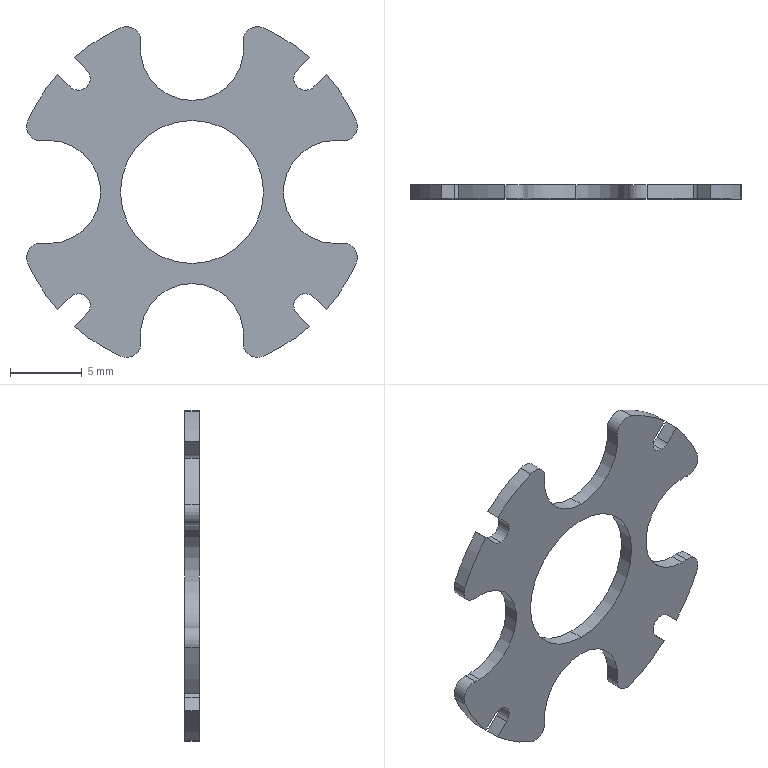Part | SolidWorks | features Extrusion 1 | 1 solid | 47 faces | box 23.109 x 1 x 23.109 mm | volume 247.856 mm3 | cylinder 37 | plane 10 | commonest cylinder face diameters 2 x12 7.2 x9 25 x8 1.65 x6 10 x2
STEP:
#1=CARTESIAN_POINT('',(0.,1.,-5.));
#2=VERTEX_POINT('',#1);
#3=CARTESIAN_POINT('',(0.,1.,5.));
#4=VERTEX_POINT('',#3);
#5=CARTESIAN_POINT('',(0.,1.,0.));
#6=DIRECTION('',(0.,1.,0.));
#7=DIRECTION('',(0.,0.,1.));
#8=AXIS2_PLACEMENT_3D('',#5,#6,#7);
#9=CIRCLE('',#8,5.);
#10=EDGE_CURVE('',#2,#4,#9,.T.);
#11=ORIENTED_EDGE('',*,*,#10,.T.);
#12=CARTESIAN_POINT('',(0.,0.,5.));
#13=VERTEX_POINT('',#12);
#14=CARTESIAN_POINT('',(0.,1.,5.));
#15=DIRECTION('',(0.,-1.,0.));
#16=VECTOR('',#15,1000.);
#17=LINE('',#14,#16);
#18=EDGE_CURVE('',#4,#13,#17,.T.);
#19=ORIENTED_EDGE('',*,*,#18,.T.);
#20=CARTESIAN_POINT('',(0.,0.,-5.));
#21=VERTEX_POINT('',#20);
#22=CARTESIAN_POINT('',(0.,0.,0.));
#23=DIRECTION('',(0.,1.,0.));
#24=DIRECTION('',(0.,0.,1.));
#25=AXIS2_PLACEMENT_3D('',#22,#23,#24);
#26=CIRCLE('',#25,5.);
#27=EDGE_CURVE('',#21,#13,#26,.T.);
#28=ORIENTED_EDGE('',*,*,#27,.F.);
#29=CARTESIAN_POINT('',(0.,1.,-5.));
#30=DIRECTION('',(0.,-1.,0.));
#31=VECTOR('',#30,1000.);
#32=LINE('',#29,#31);
#33=EDGE_CURVE('',#2,#21,#32,.T.);
#34=ORIENTED_EDGE('',*,*,#33,.F.);
#35=EDGE_LOOP('',(#11,#19,#28,#34));
#36=FACE_OUTER_BOUND('',#35,.T.);
#37=CARTESIAN_POINT('',(0.,1.,0.));
#38=DIRECTION('',(0.,-1.,0.));
#39=DIRECTION('',(0.,0.,-1.));
#40=AXIS2_PLACEMENT_3D('',#37,#38,#39);
#41=CYLINDRICAL_SURFACE('',#40,5.);
#42=ADVANCED_FACE('',(#36),#41,.F.);
#43=CARTESIAN_POINT('',(-7.937,1.,7.112));
#44=VERTEX_POINT('',#43);
#45=CARTESIAN_POINT('',(-7.354,1.,8.521));
#46=VERTEX_POINT('',#45);
#47=CARTESIAN_POINT('',(-7.937,1.,7.937));
#48=DIRECTION('',(0.,-1.,0.));
#49=DIRECTION('',(0.,0.,1.));
#50=AXIS2_PLACEMENT_3D('',#47,#48,#49);
#51=CIRCLE('',#50,0.825);
#52=EDGE_CURVE('',#44,#46,#51,.T.);
#53=ORIENTED_EDGE('',*,*,#52,.F.);
#54=CARTESIAN_POINT('',(-7.937,0.,7.112));
#55=VERTEX_POINT('',#54);
#56=CARTESIAN_POINT('',(-7.937,1.,7.112));
#57=DIRECTION('',(0.,-1.,0.));
#58=VECTOR('',#57,1000.);
#59=LINE('',#56,#58);
#60=EDGE_CURVE('',#44,#55,#59,.T.);
#61=ORIENTED_EDGE('',*,*,#60,.T.);
#62=CARTESIAN_POINT('',(-7.354,0.,8.521));
#63=VERTEX_POINT('',#62);
#64=CARTESIAN_POINT('',(-7.937,0.,7.937));
#65=DIRECTION('',(0.,-1.,0.));
#66=DIRECTION('',(0.,0.,1.));
#67=AXIS2_PLACEMENT_3D('',#64,#65,#66);
#68=CIRCLE('',#67,0.825);
#69=EDGE_CURVE('',#55,#63,#68,.T.);
#70=ORIENTED_EDGE('',*,*,#69,.T.);
#71=CARTESIAN_POINT('',(-7.354,1.,8.521));
#72=DIRECTION('',(0.,-1.,0.));
#73=VECTOR('',#72,1000.);
#74=LINE('',#71,#73);
#75=EDGE_CURVE('',#46,#63,#74,.T.);
#76=ORIENTED_EDGE('',*,*,#75,.F.);
#77=EDGE_LOOP('',(#53,#61,#70,#76));
#78=FACE_OUTER_BOUND('',#77,.T.);
#79=CARTESIAN_POINT('',(-7.937,1.,7.937));
#80=DIRECTION('',(0.,-1.,0.));
#81=DIRECTION('',(0.,0.,-1.));
#82=AXIS2_PLACEMENT_3D('',#79,#80,#81);
#83=CYLINDRICAL_SURFACE('',#82,0.825);
#84=ADVANCED_FACE('',(#78),#83,.F.);
#85=CARTESIAN_POINT('',(-10.555,1.,3.566));
#86=VERTEX_POINT('',#85);
#87=CARTESIAN_POINT('',(-11.472,1.,4.964));
#88=VERTEX_POINT('',#87);
#89=CARTESIAN_POINT('',(-10.555,1.,4.566));
#90=DIRECTION('',(0.,1.,0.));
#91=DIRECTION('',(0.,0.,1.));
#92=AXIS2_PLACEMENT_3D('',#89,#90,#91);
#93=CIRCLE('',#92,1.);
#94=EDGE_CURVE('',#86,#88,#93,.T.);
#95=ORIENTED_EDGE('',*,*,#94,.F.);
#96=CARTESIAN_POINT('',(-10.555,0.,3.566));
#97=VERTEX_POINT('',#96);
#98=CARTESIAN_POINT('',(-10.555,1.,3.566));
#99=DIRECTION('',(0.,-1.,0.));
#100=VECTOR('',#99,1000.);
#101=LINE('',#98,#100);
#102=EDGE_CURVE('',#86,#97,#101,.T.);
#103=ORIENTED_EDGE('',*,*,#102,.T.);
#104=CARTESIAN_POINT('',(-11.472,0.,4.964));
#105=VERTEX_POINT('',#104);
#106=CARTESIAN_POINT('',(-10.555,0.,4.566));
#107=DIRECTION('',(0.,1.,0.));
#108=DIRECTION('',(0.,0.,1.));
#109=AXIS2_PLACEMENT_3D('',#106,#107,#108);
#110=CIRCLE('',#109,1.);
#111=EDGE_CURVE('',#97,#105,#110,.T.);
#112=ORIENTED_EDGE('',*,*,#111,.T.);
#113=CARTESIAN_POINT('',(-11.472,1.,4.964));
#114=DIRECTION('',(0.,-1.,0.));
#115=VECTOR('',#114,1000.);
#116=LINE('',#113,#115);
#117=EDGE_CURVE('',#88,#105,#116,.T.);
#118=ORIENTED_EDGE('',*,*,#117,.F.);
#119=EDGE_LOOP('',(#95,#103,#112,#118));
#120=FACE_OUTER_BOUND('',#119,.T.);
#121=CARTESIAN_POINT('',(-10.555,1.,4.566));
#122=DIRECTION('',(0.,-1.,0.));
#123=DIRECTION('',(0.,0.,-1.));
#124=AXIS2_PLACEMENT_3D('',#121,#122,#123);
#125=CYLINDRICAL_SURFACE('',#124,1.);
#126=ADVANCED_FACE('',(#120),#125,.T.);
#127=CARTESIAN_POINT('',(-10.,1.,3.6));
#128=VERTEX_POINT('',#127);
#129=CARTESIAN_POINT('',(-10.434,1.,3.574));
#130=VERTEX_POINT('',#129);
#131=CARTESIAN_POINT('',(-10.,1.,0.));
#132=DIRECTION('',(0.,-1.,0.));
#133=DIRECTION('',(0.,0.,1.));
#134=AXIS2_PLACEMENT_3D('',#131,#132,#133);
#135=CIRCLE('',#134,3.6);
#136=EDGE_CURVE('',#128,#130,#135,.T.);
#137=ORIENTED_EDGE('',*,*,#136,.F.);
#138=CARTESIAN_POINT('',(-10.,0.,3.6));
#139=VERTEX_POINT('',#138);
#140=CARTESIAN_POINT('',(-10.,1.,3.6));
#141=DIRECTION('',(0.,-1.,0.));
#142=VECTOR('',#141,1000.);
#143=LINE('',#140,#142);
#144=EDGE_CURVE('',#128,#139,#143,.T.);
#145=ORIENTED_EDGE('',*,*,#144,.T.);
#146=CARTESIAN_POINT('',(-10.434,0.,3.574));
#147=VERTEX_POINT('',#146);
#148=CARTESIAN_POINT('',(-10.,0.,0.));
#149=DIRECTION('',(0.,-1.,0.));
#150=DIRECTION('',(0.,0.,1.));
#151=AXIS2_PLACEMENT_3D('',#148,#149,#150);
#152=CIRCLE('',#151,3.6);
#153=EDGE_CURVE('',#139,#147,#152,.T.);
#154=ORIENTED_EDGE('',*,*,#153,.T.);
#155=CARTESIAN_POINT('',(-10.434,1.,3.574));
#156=DIRECTION('',(0.,-1.,0.));
#157=VECTOR('',#156,1000.);
#158=LINE('',#155,#157);
#159=EDGE_CURVE('',#130,#147,#158,.T.);
#160=ORIENTED_EDGE('',*,*,#159,.F.);
#161=EDGE_LOOP('',(#137,#145,#154,#160));
#162=FACE_OUTER_BOUND('',#161,.T.);
#163=CARTESIAN_POINT('',(-10.,1.,0.));
#164=DIRECTION('',(0.,-1.,0.));
#165=DIRECTION('',(0.,0.,-1.));
#166=AXIS2_PLACEMENT_3D('',#163,#164,#165);
#167=CYLINDRICAL_SURFACE('',#166,3.6);
#168=ADVANCED_FACE('',(#162),#167,.F.);
#169=ORIENTED_EDGE('',*,*,#144,.F.);
#170=CARTESIAN_POINT('',(-10.,1.,-3.6));
#171=VERTEX_POINT('',#170);
#172=CARTESIAN_POINT('',(-10.,1.,0.));
#173=DIRECTION('',(0.,-1.,0.));
#174=DIRECTION('',(0.,0.,1.));
#175=AXIS2_PLACEMENT_3D('',#172,#173,#174);
#176=CIRCLE('',#175,3.6);
#177=EDGE_CURVE('',#171,#128,#176,.T.);
#178=ORIENTED_EDGE('',*,*,#177,.F.);
#179=CARTESIAN_POINT('',(-10.,0.,-3.6));
#180=VERTEX_POINT('',#179);
#181=CARTESIAN_POINT('',(-10.,1.,-3.6));
#182=DIRECTION('',(0.,-1.,0.));
#183=VECTOR('',#182,1000.);
#184=LINE('',#181,#183);
#185=EDGE_CURVE('',#171,#180,#184,.T.);
#186=ORIENTED_EDGE('',*,*,#185,.T.);
#187=CARTESIAN_POINT('',(-10.,0.,0.));
#188=DIRECTION('',(0.,-1.,0.));
#189=DIRECTION('',(0.,0.,1.));
#190=AXIS2_PLACEMENT_3D('',#187,#188,#189);
#191=CIRCLE('',#190,3.6);
#192=EDGE_CURVE('',#180,#139,#191,.T.);
#193=ORIENTED_EDGE('',*,*,#192,.T.);
#194=EDGE_LOOP('',(#169,#178,#186,#193));
#195=FACE_OUTER_BOUND('',#194,.T.);
#196=CARTESIAN_POINT('',(-10.,1.,0.));
#197=DIRECTION('',(0.,-1.,0.));
#198=DIRECTION('',(0.,0.,-1.));
#199=AXIS2_PLACEMENT_3D('',#196,#197,#198);
#200=CYLINDRICAL_SURFACE('',#199,3.6);
#201=ADVANCED_FACE('',(#195),#200,.F.);
#202=CARTESIAN_POINT('',(-4.566,1.,-11.555));
#203=VERTEX_POINT('',#202);
#204=CARTESIAN_POINT('',(-4.964,1.,-11.472));
#205=VERTEX_POINT('',#204);
#206=CARTESIAN_POINT('',(-4.566,1.,-10.554));
#207=DIRECTION('',(0.,1.,0.));
#208=DIRECTION('',(0.,0.,1.));
#209=AXIS2_PLACEMENT_3D('',#206,#207,#208);
#210=CIRCLE('',#209,1.);
#211=EDGE_CURVE('',#203,#205,#210,.T.);
#212=ORIENTED_EDGE('',*,*,#211,.F.);
#213=CARTESIAN_POINT('',(-4.566,0.,-11.555));
#214=VERTEX_POINT('',#213);
#215=CARTESIAN_POINT('',(-4.566,1.,-11.554));
#216=DIRECTION('',(0.,-1.,0.));
#217=VECTOR('',#216,1000.);
#218=LINE('',#215,#217);
#219=EDGE_CURVE('',#203,#214,#218,.T.);
#220=ORIENTED_EDGE('',*,*,#219,.T.);
#221=CARTESIAN_POINT('',(-4.964,0.,-11.472));
#222=VERTEX_POINT('',#221);
#223=CARTESIAN_POINT('',(-4.566,0.,-10.554));
#224=DIRECTION('',(0.,1.,0.));
#225=DIRECTION('',(0.,0.,1.));
#226=AXIS2_PLACEMENT_3D('',#223,#224,#225);
#227=CIRCLE('',#226,1.);
#228=EDGE_CURVE('',#214,#222,#227,.T.);
#229=ORIENTED_EDGE('',*,*,#228,.T.);
#230=CARTESIAN_POINT('',(-4.964,1.,-11.472));
#231=DIRECTION('',(0.,-1.,0.));
#232=VECTOR('',#231,1000.);
#233=LINE('',#230,#232);
#234=EDGE_CURVE('',#205,#222,#233,.T.);
#235=ORIENTED_EDGE('',*,*,#234,.F.);
#236=EDGE_LOOP('',(#212,#220,#229,#235));
#237=FACE_OUTER_BOUND('',#236,.T.);
#238=CARTESIAN_POINT('',(-4.566,1.,-10.554));
#239=DIRECTION('',(0.,-1.,0.));
#240=DIRECTION('',(0.,0.,-1.));
#241=AXIS2_PLACEMENT_3D('',#238,#239,#240);
#242=CYLINDRICAL_SURFACE('',#241,1.);
#243=ADVANCED_FACE('',(#237),#242,.T.);
#244=CARTESIAN_POINT('',(4.566,1.,-11.555));
#245=VERTEX_POINT('',#244);
#246=CARTESIAN_POINT('',(3.574,1.,-10.434));
#247=VERTEX_POINT('',#246);
#248=CARTESIAN_POINT('',(4.566,1.,-10.554));
#249=DIRECTION('',(0.,1.,0.));
#250=DIRECTION('',(0.,0.,1.));
#251=AXIS2_PLACEMENT_3D('',#248,#249,#250);
#252=CIRCLE('',#251,1.);
#253=EDGE_CURVE('',#245,#247,#252,.T.);
#254=ORIENTED_EDGE('',*,*,#253,.F.);
#255=CARTESIAN_POINT('',(4.566,0.,-11.555));
#256=VERTEX_POINT('',#255);
#257=CARTESIAN_POINT('',(4.566,1.,-11.554));
#258=DIRECTION('',(0.,-1.,0.));
#259=VECTOR('',#258,1000.);
#260=LINE('',#257,#259);
#261=EDGE_CURVE('',#245,#256,#260,.T.);
#262=ORIENTED_EDGE('',*,*,#261,.T.);
#263=CARTESIAN_POINT('',(3.574,0.,-10.434));
#264=VERTEX_POINT('',#263);
#265=CARTESIAN_POINT('',(4.566,0.,-10.555));
#266=DIRECTION('',(0.,1.,0.));
#267=DIRECTION('',(0.,0.,1.));
#268=AXIS2_PLACEMENT_3D('',#265,#266,#267);
#269=CIRCLE('',#268,1.);
#270=EDGE_CURVE('',#256,#264,#269,.T.);
#271=ORIENTED_EDGE('',*,*,#270,.T.);
#272=CARTESIAN_POINT('',(3.574,1.,-10.434));
#273=DIRECTION('',(0.,-1.,0.));
#274=VECTOR('',#273,1000.);
#275=LINE('',#272,#274);
#276=EDGE_CURVE('',#247,#264,#275,.T.);
#277=ORIENTED_EDGE('',*,*,#276,.F.);
#278=EDGE_LOOP('',(#254,#262,#271,#277));
#279=FACE_OUTER_BOUND('',#278,.T.);
#280=CARTESIAN_POINT('',(4.566,1.,-10.554));
#281=DIRECTION('',(0.,-1.,0.));
#282=DIRECTION('',(0.,0.,-1.));
#283=AXIS2_PLACEMENT_3D('',#280,#281,#282);
#284=CYLINDRICAL_SURFACE('',#283,1.);
#285=ADVANCED_FACE('',(#279),#284,.T.);
#286=CARTESIAN_POINT('',(10.,1.,3.6));
#287=VERTEX_POINT('',#286);
#288=CARTESIAN_POINT('',(10.,1.,-3.6));
#289=VERTEX_POINT('',#288);
#290=CARTESIAN_POINT('',(10.,1.,0.));
#291=DIRECTION('',(0.,-1.,0.));
#292=DIRECTION('',(0.,0.,1.));
#293=AXIS2_PLACEMENT_3D('',#290,#291,#292);
#294=CIRCLE('',#293,3.6);
#295=EDGE_CURVE('',#287,#289,#294,.T.);
#296=ORIENTED_EDGE('',*,*,#295,.F.);
#297=CARTESIAN_POINT('',(10.,0.,3.6));
#298=VERTEX_POINT('',#297);
#299=CARTESIAN_POINT('',(10.,1.,3.6));
#300=DIRECTION('',(0.,-1.,0.));
#301=VECTOR('',#300,1000.);
#302=LINE('',#299,#301);
#303=EDGE_CURVE('',#287,#298,#302,.T.);
#304=ORIENTED_EDGE('',*,*,#303,.T.);
#305=CARTESIAN_POINT('',(10.,0.,-3.6));
#306=VERTEX_POINT('',#305);
#307=CARTESIAN_POINT('',(10.,0.,0.));
#308=DIRECTION('',(0.,-1.,0.));
#309=DIRECTION('',(0.,0.,1.));
#310=AXIS2_PLACEMENT_3D('',#307,#308,#309);
#311=CIRCLE('',#310,3.6);
#312=EDGE_CURVE('',#298,#306,#311,.T.);
#313=ORIENTED_EDGE('',*,*,#312,.T.);
#314=CARTESIAN_POINT('',(10.,1.,-3.6));
#315=DIRECTION('',(0.,-1.,0.));
#316=VECTOR('',#315,1000.);
#317=LINE('',#314,#316);
#318=EDGE_CURVE('',#289,#306,#317,.T.);
#319=ORIENTED_EDGE('',*,*,#318,.F.);
#320=EDGE_LOOP('',(#296,#304,#313,#319));
#321=FACE_OUTER_BOUND('',#320,.T.);
#322=CARTESIAN_POINT('',(10.,1.,0.));
#323=DIRECTION('',(0.,-1.,0.));
#324=DIRECTION('',(0.,0.,-1.));
#325=AXIS2_PLACEMENT_3D('',#322,#323,#324);
#326=CYLINDRICAL_SURFACE('',#325,3.6);
#327=ADVANCED_FACE('',(#321),#326,.F.);
#328=CARTESIAN_POINT('',(10.434,1.,-3.574));
#329=VERTEX_POINT('',#328);
#330=CARTESIAN_POINT('',(10.,1.,0.));
#331=DIRECTION('',(0.,-1.,0.));
#332=DIRECTION('',(0.,0.,1.));
#333=AXIS2_PLACEMENT_3D('',#330,#331,#332);
#334=CIRCLE('',#333,3.6);
#335=EDGE_CURVE('',#289,#329,#334,.T.);
#336=ORIENTED_EDGE('',*,*,#335,.F.);
#337=ORIENTED_EDGE('',*,*,#318,.T.);
#338=CARTESIAN_POINT('',(10.434,0.,-3.574));
#339=VERTEX_POINT('',#338);
#340=CARTESIAN_POINT('',(10.,0.,0.));
#341=DIRECTION('',(0.,-1.,0.));
#342=DIRECTION('',(0.,0.,1.));
#343=AXIS2_PLACEMENT_3D('',#340,#341,#342);
#344=CIRCLE('',#343,3.6);
#345=EDGE_CURVE('',#306,#339,#344,.T.);
#346=ORIENTED_EDGE('',*,*,#345,.T.);
#347=CARTESIAN_POINT('',(10.434,1.,-3.574));
#348=DIRECTION('',(0.,-1.,0.));
#349=VECTOR('',#348,1000.);
#350=LINE('',#347,#349);
#351=EDGE_CURVE('',#329,#339,#350,.T.);
#352=ORIENTED_EDGE('',*,*,#351,.F.);
#353=EDGE_LOOP('',(#336,#337,#346,#352));
#354=FACE_OUTER_BOUND('',#353,.T.);
#355=CARTESIAN_POINT('',(10.,1.,0.));
#356=DIRECTION('',(0.,-1.,0.));
#357=DIRECTION('',(0.,0.,-1.));
#358=AXIS2_PLACEMENT_3D('',#355,#356,#357);
#359=CYLINDRICAL_SURFACE('',#358,3.6);
#360=ADVANCED_FACE('',(#354),#359,.F.);
#361=CARTESIAN_POINT('',(10.554,1.,3.566));
#362=VERTEX_POINT('',#361);
#363=CARTESIAN_POINT('',(10.434,1.,3.574));
#364=VERTEX_POINT('',#363);
#365=CARTESIAN_POINT('',(10.554,1.,4.566));
#366=DIRECTION('',(0.,1.,0.));
#367=DIRECTION('',(0.,0.,1.));
#368=AXIS2_PLACEMENT_3D('',#365,#366,#367);
#369=CIRCLE('',#368,1.);
#370=EDGE_CURVE('',#362,#364,#369,.T.);
#371=ORIENTED_EDGE('',*,*,#370,.F.);
#372=CARTESIAN_POINT('',(10.554,0.,3.566));
#373=VERTEX_POINT('',#372);
#374=CARTESIAN_POINT('',(10.554,1.,3.566));
#375=DIRECTION('',(0.,-1.,0.));
#376=VECTOR('',#375,1000.);
#377=LINE('',#374,#376);
#378=EDGE_CURVE('',#362,#373,#377,.T.);
#379=ORIENTED_EDGE('',*,*,#378,.T.);
#380=CARTESIAN_POINT('',(10.434,0.,3.574));
#381=VERTEX_POINT('',#380);
#382=CARTESIAN_POINT('',(10.555,0.,4.566));
#383=DIRECTION('',(0.,1.,0.));
#384=DIRECTION('',(0.,0.,1.));
#385=AXIS2_PLACEMENT_3D('',#382,#383,#384);
#386=CIRCLE('',#385,1.);
#387=EDGE_CURVE('',#373,#381,#386,.T.);
#388=ORIENTED_EDGE('',*,*,#387,.T.);
#389=CARTESIAN_POINT('',(10.434,1.,3.574));
#390=DIRECTION('',(0.,-1.,0.));
#391=VECTOR('',#390,1000.);
#392=LINE('',#389,#391);
#393=EDGE_CURVE('',#364,#381,#392,.T.);
#394=ORIENTED_EDGE('',*,*,#393,.F.);
#395=EDGE_LOOP('',(#371,#379,#388,#394));
#396=FACE_OUTER_BOUND('',#395,.T.);
#397=CARTESIAN_POINT('',(10.554,1.,4.566));
#398=DIRECTION('',(0.,-1.,0.));
#399=DIRECTION('',(0.,0.,-1.));
#400=AXIS2_PLACEMENT_3D('',#397,#398,#399);
#401=CYLINDRICAL_SURFACE('',#400,1.);
#402=ADVANCED_FACE('',(#396),#401,.T.);
#403=CARTESIAN_POINT('',(7.937,1.,7.112));
#404=VERTEX_POINT('',#403);
#405=CARTESIAN_POINT('',(8.521,1.,7.354));
#406=VERTEX_POINT('',#405);
#407=CARTESIAN_POINT('',(7.937,1.,7.937));
#408=DIRECTION('',(0.,-1.,0.));
#409=DIRECTION('',(0.,0.,1.));
#410=AXIS2_PLACEMENT_3D('',#407,#408,#409);
#411=CIRCLE('',#410,0.825);
#412=EDGE_CURVE('',#404,#406,#411,.T.);
#413=ORIENTED_EDGE('',*,*,#412,.F.);
#414=CARTESIAN_POINT('',(7.937,0.,7.112));
#415=VERTEX_POINT('',#414);
#416=CARTESIAN_POINT('',(7.937,1.,7.112));
#417=DIRECTION('',(0.,-1.,0.));
#418=VECTOR('',#417,1000.);
#419=LINE('',#416,#418);
#420=EDGE_CURVE('',#404,#415,#419,.T.);
#421=ORIENTED_EDGE('',*,*,#420,.T.);
#422=CARTESIAN_POINT('',(8.521,0.,7.354));
#423=VERTEX_POINT('',#422);
#424=CARTESIAN_POINT('',(7.937,0.,7.937));
#425=DIRECTION('',(0.,-1.,0.));
#426=DIRECTION('',(0.,0.,1.));
#427=AXIS2_PLACEMENT_3D('',#424,#425,#426);
#428=CIRCLE('',#427,0.825);
#429=EDGE_CURVE('',#415,#423,#428,.T.);
#430=ORIENTED_EDGE('',*,*,#429,.T.);
#431=CARTESIAN_POINT('',(8.521,1.,7.354));
#432=DIRECTION('',(0.,-1.,0.));
#433=VECTOR('',#432,1000.);
#434=LINE('',#431,#433);
#435=EDGE_CURVE('',#406,#423,#434,.T.);
#436=ORIENTED_EDGE('',*,*,#435,.F.);
#437=EDGE_LOOP('',(#413,#421,#430,#436));
#438=FACE_OUTER_BOUND('',#437,.T.);
#439=CARTESIAN_POINT('',(7.937,1.,7.937));
#440=DIRECTION('',(0.,-1.,0.));
#441=DIRECTION('',(0.,0.,-1.));
#442=AXIS2_PLACEMENT_3D('',#439,#440,#441);
#443=CYLINDRICAL_SURFACE('',#442,0.825);
#444=ADVANCED_FACE('',(#438),#443,.F.);
#445=CARTESIAN_POINT('',(0.,1.,6.4));
#446=VERTEX_POINT('',#445);
#447=CARTESIAN_POINT('',(3.574,1.,10.434));
#448=VERTEX_POINT('',#447);
#449=CARTESIAN_POINT('',(0.,1.,10.));
#450=DIRECTION('',(0.,-1.,0.));
#451=DIRECTION('',(0.,0.,1.));
#452=AXIS2_PLACEMENT_3D('',#449,#450,#451);
#453=CIRCLE('',#452,3.6);
#454=EDGE_CURVE('',#446,#448,#453,.T.);
#455=ORIENTED_EDGE('',*,*,#454,.F.);
#456=CARTESIAN_POINT('',(0.,0.,6.4));
#457=VERTEX_POINT('',#456);
#458=CARTESIAN_POINT('',(0.,1.,6.4));
#459=DIRECTION('',(0.,-1.,0.));
#460=VECTOR('',#459,1000.);
#461=LINE('',#458,#460);
#462=EDGE_CURVE('',#446,#457,#461,.T.);
#463=ORIENTED_EDGE('',*,*,#462,.T.);
#464=CARTESIAN_POINT('',(3.574,0.,10.434));
#465=VERTEX_POINT('',#464);
#466=CARTESIAN_POINT('',(0.,0.,10.));
#467=DIRECTION('',(0.,-1.,0.));
#468=DIRECTION('',(0.,0.,1.));
#469=AXIS2_PLACEMENT_3D('',#466,#467,#468);
#470=CIRCLE('',#469,3.6);
#471=EDGE_CURVE('',#457,#465,#470,.T.);
#472=ORIENTED_EDGE('',*,*,#471,.T.);
#473=CARTESIAN_POINT('',(3.574,1.,10.434));
#474=DIRECTION('',(0.,-1.,0.));
#475=VECTOR('',#474,1000.);
#476=LINE('',#473,#475);
#477=EDGE_CURVE('',#448,#465,#476,.T.);
#478=ORIENTED_EDGE('',*,*,#477,.F.);
#479=EDGE_LOOP('',(#455,#463,#472,#478));
#480=FACE_OUTER_BOUND('',#479,.T.);
#481=CARTESIAN_POINT('',(0.,1.,10.));
#482=DIRECTION('',(0.,-1.,0.));
#483=DIRECTION('',(0.,0.,-1.));
#484=AXIS2_PLACEMENT_3D('',#481,#482,#483);
#485=CYLINDRICAL_SURFACE('',#484,3.6);
#486=ADVANCED_FACE('',(#480),#485,.F.);
#487=CARTESIAN_POINT('',(-8.236,1.,9.403));
#488=VERTEX_POINT('',#487);
#489=CARTESIAN_POINT('',(-4.964,1.,11.472));
#490=VERTEX_POINT('',#489);
#491=CARTESIAN_POINT('',(0.,1.,0.));
#492=DIRECTION('',(0.,1.,0.));
#493=DIRECTION('',(0.,0.,1.));
#494=AXIS2_PLACEMENT_3D('',#491,#492,#493);
#495=CIRCLE('',#494,12.5);
#496=EDGE_CURVE('',#488,#490,#495,.T.);
#497=ORIENTED_EDGE('',*,*,#496,.T.);
#498=CARTESIAN_POINT('',(-3.574,1.,10.434));
#499=VERTEX_POINT('',#498);
#500=CARTESIAN_POINT('',(-4.566,1.,10.555));
#501=DIRECTION('',(0.,1.,0.));
#502=DIRECTION('',(0.,0.,1.));
#503=AXIS2_PLACEMENT_3D('',#500,#501,#502);
#504=CIRCLE('',#503,1.);
#505=EDGE_CURVE('',#490,#499,#504,.T.);
#506=ORIENTED_EDGE('',*,*,#505,.T.);
#507=CARTESIAN_POINT('',(0.,1.,10.));
#508=DIRECTION('',(0.,-1.,0.));
#509=DIRECTION('',(0.,0.,1.));
#510=AXIS2_PLACEMENT_3D('',#507,#508,#509);
#511=CIRCLE('',#510,3.6);
#512=EDGE_CURVE('',#499,#446,#511,.T.);
#513=ORIENTED_EDGE('',*,*,#512,.T.);
#514=ORIENTED_EDGE('',*,*,#454,.T.);
#515=CARTESIAN_POINT('',(4.964,1.,11.472));
#516=VERTEX_POINT('',#515);
#517=CARTESIAN_POINT('',(4.566,1.,10.555));
#518=DIRECTION('',(0.,1.,0.));
#519=DIRECTION('',(0.,0.,1.));
#520=AXIS2_PLACEMENT_3D('',#517,#518,#519);
#521=CIRCLE('',#520,1.);
#522=EDGE_CURVE('',#448,#516,#521,.T.);
#523=ORIENTED_EDGE('',*,*,#522,.T.);
#524=CARTESIAN_POINT('',(8.236,1.,9.403));
#525=VERTEX_POINT('',#524);
#526=CARTESIAN_POINT('',(0.,1.,0.));
#527=DIRECTION('',(0.,1.,0.));
#528=DIRECTION('',(0.,0.,1.));
#529=AXIS2_PLACEMENT_3D('',#526,#527,#528);
#530=CIRCLE('',#529,12.5);
#531=EDGE_CURVE('',#516,#525,#530,.T.);
#532=ORIENTED_EDGE('',*,*,#531,.T.);
#533=CARTESIAN_POINT('',(7.354,1.,8.521));
#534=VERTEX_POINT('',#533);
#535=CARTESIAN_POINT('',(7.354,1.,8.521));
#536=DIRECTION('',(-0.7071,0.,-0.7071));
#537=VECTOR('',#536,1000.);
#538=LINE('',#535,#537);
#539=EDGE_CURVE('',#525,#534,#538,.T.);
#540=ORIENTED_EDGE('',*,*,#539,.T.);
#541=CARTESIAN_POINT('',(7.937,1.,7.937));
#542=DIRECTION('',(0.,-1.,0.));
#543=DIRECTION('',(0.,0.,1.));
#544=AXIS2_PLACEMENT_3D('',#541,#542,#543);
#545=CIRCLE('',#544,0.825);
#546=EDGE_CURVE('',#534,#404,#545,.T.);
#547=ORIENTED_EDGE('',*,*,#546,.T.);
#548=ORIENTED_EDGE('',*,*,#412,.T.);
#549=CARTESIAN_POINT('',(9.403,1.,8.236));
#550=VERTEX_POINT('',#549);
#551=CARTESIAN_POINT('',(8.521,1.,7.354));
#552=DIRECTION('',(0.7071,0.,0.7071));
#553=VECTOR('',#552,1000.);
#554=LINE('',#551,#553);
#555=EDGE_CURVE('',#406,#550,#554,.T.);
#556=ORIENTED_EDGE('',*,*,#555,.T.);
#557=CARTESIAN_POINT('',(11.472,1.,4.964));
#558=VERTEX_POINT('',#557);
#559=CARTESIAN_POINT('',(0.,1.,0.));
#560=DIRECTION('',(0.,1.,0.));
#561=DIRECTION('',(0.,0.,1.));
#562=AXIS2_PLACEMENT_3D('',#559,#560,#561);
#563=CIRCLE('',#562,12.5);
#564=EDGE_CURVE('',#550,#558,#563,.T.);
#565=ORIENTED_EDGE('',*,*,#564,.T.);
#566=CARTESIAN_POINT('',(10.554,1.,4.566));
#567=DIRECTION('',(0.,1.,0.));
#568=DIRECTION('',(0.,0.,1.));
#569=AXIS2_PLACEMENT_3D('',#566,#567,#568);
#570=CIRCLE('',#569,1.);
#571=EDGE_CURVE('',#558,#362,#570,.T.);
#572=ORIENTED_EDGE('',*,*,#571,.T.);
#573=ORIENTED_EDGE('',*,*,#370,.T.);
#574=CARTESIAN_POINT('',(10.,1.,0.));
#575=DIRECTION('',(0.,-1.,0.));
#576=DIRECTION('',(0.,0.,1.));
#577=AXIS2_PLACEMENT_3D('',#574,#575,#576);
#578=CIRCLE('',#577,3.6);
#579=EDGE_CURVE('',#364,#287,#578,.T.);
#580=ORIENTED_EDGE('',*,*,#579,.T.);
#581=ORIENTED_EDGE('',*,*,#295,.T.);
#582=ORIENTED_EDGE('',*,*,#335,.T.);
#583=CARTESIAN_POINT('',(11.472,1.,-4.964));
#584=VERTEX_POINT('',#583);
#585=CARTESIAN_POINT('',(10.554,1.,-4.566));
#586=DIRECTION('',(0.,1.,0.));
#587=DIRECTION('',(0.,0.,1.));
#588=AXIS2_PLACEMENT_3D('',#585,#586,#587);
#589=CIRCLE('',#588,1.);
#590=EDGE_CURVE('',#329,#584,#589,.T.);
#591=ORIENTED_EDGE('',*,*,#590,.T.);
#592=CARTESIAN_POINT('',(9.403,1.,-8.236));
#593=VERTEX_POINT('',#592);
#594=CARTESIAN_POINT('',(0.,1.,0.));
#595=DIRECTION('',(0.,1.,0.));
#596=DIRECTION('',(0.,0.,-1.));
#597=AXIS2_PLACEMENT_3D('',#594,#595,#596);
#598=CIRCLE('',#597,12.5);
#599=EDGE_CURVE('',#584,#593,#598,.T.);
#600=ORIENTED_EDGE('',*,*,#599,.T.);
#601=CARTESIAN_POINT('',(8.521,1.,-7.354));
#602=VERTEX_POINT('',#601);
#603=CARTESIAN_POINT('',(8.521,1.,-7.354));
#604=DIRECTION('',(-0.7071,0.,0.7071));
#605=VECTOR('',#604,1000.);
#606=LINE('',#603,#605);
#607=EDGE_CURVE('',#593,#602,#606,.T.);
#608=ORIENTED_EDGE('',*,*,#607,.T.);
#609=CARTESIAN_POINT('',(7.354,1.,-8.521));
#610=VERTEX_POINT('',#609);
#611=CARTESIAN_POINT('',(7.937,1.,-7.937));
#612=DIRECTION('',(0.,-1.,0.));
#613=DIRECTION('',(0.,0.,1.));
#614=AXIS2_PLACEMENT_3D('',#611,#612,#613);
#615=CIRCLE('',#614,0.825);
#616=EDGE_CURVE('',#602,#610,#615,.T.);
#617=ORIENTED_EDGE('',*,*,#616,.T.);
#618=CARTESIAN_POINT('',(8.236,1.,-9.403));
#619=VERTEX_POINT('',#618);
#620=CARTESIAN_POINT('',(7.354,1.,-8.521));
#621=DIRECTION('',(0.7071,0.,-0.7071));
#622=VECTOR('',#621,1000.);
#623=LINE('',#620,#622);
#624=EDGE_CURVE('',#610,#619,#623,.T.);
#625=ORIENTED_EDGE('',*,*,#624,.T.);
#626=CARTESIAN_POINT('',(4.964,1.,-11.472));
#627=VERTEX_POINT('',#626);
#628=CARTESIAN_POINT('',(0.,1.,0.));
#629=DIRECTION('',(0.,1.,0.));
#630=DIRECTION('',(0.,0.,-1.));
#631=AXIS2_PLACEMENT_3D('',#628,#629,#630);
#632=CIRCLE('',#631,12.5);
#633=EDGE_CURVE('',#619,#627,#632,.T.);
#634=ORIENTED_EDGE('',*,*,#633,.T.);
#635=CARTESIAN_POINT('',(4.566,1.,-10.554));
#636=DIRECTION('',(0.,1.,0.));
#637=DIRECTION('',(0.,0.,1.));
#638=AXIS2_PLACEMENT_3D('',#635,#636,#637);
#639=CIRCLE('',#638,1.);
#640=EDGE_CURVE('',#627,#245,#639,.T.);
#641=ORIENTED_EDGE('',*,*,#640,.T.);
#642=ORIENTED_EDGE('',*,*,#253,.T.);
#643=CARTESIAN_POINT('',(-3.574,1.,-10.434));
#644=VERTEX_POINT('',#643);
#645=CARTESIAN_POINT('',(0.,1.,-10.));
#646=DIRECTION('',(0.,-1.,0.));
#647=DIRECTION('',(0.,0.,1.));
#648=AXIS2_PLACEMENT_3D('',#645,#646,#647);
#649=CIRCLE('',#648,3.6);
#650=EDGE_CURVE('',#247,#644,#649,.T.);
#651=ORIENTED_EDGE('',*,*,#650,.T.);
#652=CARTESIAN_POINT('',(-4.566,1.,-10.554));
#653=DIRECTION('',(0.,1.,0.));
#654=DIRECTION('',(0.,0.,1.));
#655=AXIS2_PLACEMENT_3D('',#652,#653,#654);
#656=CIRCLE('',#655,1.);
#657=EDGE_CURVE('',#644,#203,#656,.T.);
#658=ORIENTED_EDGE('',*,*,#657,.T.);
#659=ORIENTED_EDGE('',*,*,#211,.T.);
#660=CARTESIAN_POINT('',(-8.236,1.,-9.403));
#661=VERTEX_POINT('',#660);
#662=CARTESIAN_POINT('',(0.,1.,0.));
#663=DIRECTION('',(0.,1.,0.));
#664=DIRECTION('',(0.,0.,1.));
#665=AXIS2_PLACEMENT_3D('',#662,#663,#664);
#666=CIRCLE('',#665,12.5);
#667=EDGE_CURVE('',#205,#661,#666,.T.);
#668=ORIENTED_EDGE('',*,*,#667,.T.);
#669=CARTESIAN_POINT('',(-7.354,1.,-8.521));
#670=VERTEX_POINT('',#669);
#671=CARTESIAN_POINT('',(-7.354,1.,-8.521));
#672=DIRECTION('',(0.7071,0.,0.7071));
#673=VECTOR('',#672,1000.);
#674=LINE('',#671,#673);
#675=EDGE_CURVE('',#661,#670,#674,.T.);
#676=ORIENTED_EDGE('',*,*,#675,.T.);
#677=CARTESIAN_POINT('',(-8.521,1.,-7.354));
#678=VERTEX_POINT('',#677);
#679=CARTESIAN_POINT('',(-7.937,1.,-7.937));
#680=DIRECTION('',(0.,-1.,0.));
#681=DIRECTION('',(0.,0.,1.));
#682=AXIS2_PLACEMENT_3D('',#679,#680,#681);
#683=CIRCLE('',#682,0.825);
#684=EDGE_CURVE('',#670,#678,#683,.T.);
#685=ORIENTED_EDGE('',*,*,#684,.T.);
#686=CARTESIAN_POINT('',(-9.403,1.,-8.236));
#687=VERTEX_POINT('',#686);
#688=CARTESIAN_POINT('',(-8.521,1.,-7.354));
#689=DIRECTION('',(-0.7071,0.,-0.7071));
#690=VECTOR('',#689,1000.);
#691=LINE('',#688,#690);
#692=EDGE_CURVE('',#678,#687,#691,.T.);
#693=ORIENTED_EDGE('',*,*,#692,.T.);
#694=CARTESIAN_POINT('',(-11.472,1.,-4.964));
#695=VERTEX_POINT('',#694);
#696=CARTESIAN_POINT('',(0.,1.,0.));
#697=DIRECTION('',(0.,1.,0.));
#698=DIRECTION('',(0.,0.,1.));
#699=AXIS2_PLACEMENT_3D('',#696,#697,#698);
#700=CIRCLE('',#699,12.5);
#701=EDGE_CURVE('',#687,#695,#700,.T.);
#702=ORIENTED_EDGE('',*,*,#701,.T.);
#703=CARTESIAN_POINT('',(-10.434,1.,-3.574));
#704=VERTEX_POINT('',#703);
#705=CARTESIAN_POINT('',(-10.555,1.,-4.566));
#706=DIRECTION('',(0.,1.,0.));
#707=DIRECTION('',(0.,0.,1.));
#708=AXIS2_PLACEMENT_3D('',#705,#706,#707);
#709=CIRCLE('',#708,1.);
#710=EDGE_CURVE('',#695,#704,#709,.T.);
#711=ORIENTED_EDGE('',*,*,#710,.T.);
#712=CARTESIAN_POINT('',(-10.,1.,0.));
#713=DIRECTION('',(0.,-1.,0.));
#714=DIRECTION('',(0.,0.,1.));
#715=AXIS2_PLACEMENT_3D('',#712,#713,#714);
#716=CIRCLE('',#715,3.6);
#717=EDGE_CURVE('',#704,#171,#716,.T.);
#718=ORIENTED_EDGE('',*,*,#717,.T.);
#719=ORIENTED_EDGE('',*,*,#177,.T.);
#720=ORIENTED_EDGE('',*,*,#136,.T.);
#721=CARTESIAN_POINT('',(-10.555,1.,4.566));
#722=DIRECTION('',(0.,1.,0.));
#723=DIRECTION('',(0.,0.,1.));
#724=AXIS2_PLACEMENT_3D('',#721,#722,#723);
#725=CIRCLE('',#724,1.);
#726=EDGE_CURVE('',#130,#86,#725,.T.);
#727=ORIENTED_EDGE('',*,*,#726,.T.);
#728=ORIENTED_EDGE('',*,*,#94,.T.);
#729=CARTESIAN_POINT('',(-9.403,1.,8.236));
#730=VERTEX_POINT('',#729);
#731=CARTESIAN_POINT('',(0.,1.,0.));
#732=DIRECTION('',(0.,1.,0.));
#733=DIRECTION('',(0.,0.,1.));
#734=AXIS2_PLACEMENT_3D('',#731,#732,#733);
#735=CIRCLE('',#734,12.5);
#736=EDGE_CURVE('',#88,#730,#735,.T.);
#737=ORIENTED_EDGE('',*,*,#736,.T.);
#738=CARTESIAN_POINT('',(-8.521,1.,7.354));
#739=VERTEX_POINT('',#738);
#740=CARTESIAN_POINT('',(-8.521,1.,7.354));
#741=DIRECTION('',(0.7071,0.,-0.7071));
#742=VECTOR('',#741,1000.);
#743=LINE('',#740,#742);
#744=EDGE_CURVE('',#730,#739,#743,.T.);
#745=ORIENTED_EDGE('',*,*,#744,.T.);
#746=CARTESIAN_POINT('',(-7.937,1.,7.937));
#747=DIRECTION('',(0.,-1.,0.));
#748=DIRECTION('',(0.,0.,1.));
#749=AXIS2_PLACEMENT_3D('',#746,#747,#748);
#750=CIRCLE('',#749,0.825);
#751=EDGE_CURVE('',#739,#44,#750,.T.);
#752=ORIENTED_EDGE('',*,*,#751,.T.);
#753=ORIENTED_EDGE('',*,*,#52,.T.);
#754=CARTESIAN_POINT('',(-7.354,1.,8.521));
#755=DIRECTION('',(-0.7071,0.,0.7071));
#756=VECTOR('',#755,1000.);
#757=LINE('',#754,#756);
#758=EDGE_CURVE('',#46,#488,#757,.T.);
#759=ORIENTED_EDGE('',*,*,#758,.T.);
#760=EDGE_LOOP('',(#497,#506,#513,#514,#523,#532,#540,#547,#548,#556,#565,#572,#573,#580,#581,#582,#591,#600,#608,#617,#625,#634,#641,#642,#651,#658,#659,#668,#676,#685,#693,#702,#711,#718,#719,#720,#727,#728,#737,#745,#752,#753,#759));
#761=FACE_OUTER_BOUND('',#760,.T.);
#762=ORIENTED_EDGE('',*,*,#10,.F.);
#763=CARTESIAN_POINT('',(0.,1.,0.));
#764=DIRECTION('',(0.,1.,0.));
#765=DIRECTION('',(0.,0.,1.));
#766=AXIS2_PLACEMENT_3D('',#763,#764,#765);
#767=CIRCLE('',#766,5.);
#768=EDGE_CURVE('',#4,#2,#767,.T.);
#769=ORIENTED_EDGE('',*,*,#768,.F.);
#770=EDGE_LOOP('',(#762,#769));
#771=FACE_BOUND('',#770,.T.);
#772=CARTESIAN_POINT('',(0.,1.,0.));
#773=DIRECTION('',(0.,1.,0.));
#774=DIRECTION('',(0.,0.,1.));
#775=AXIS2_PLACEMENT_3D('',#772,#773,#774);
#776=PLANE('',#775);
#777=ADVANCED_FACE('',(#761,#771),#776,.T.);
#778=CARTESIAN_POINT('',(-8.236,0.,9.403));
#779=VERTEX_POINT('',#778);
#780=CARTESIAN_POINT('',(-4.964,0.,11.472));
#781=VERTEX_POINT('',#780);
#782=CARTESIAN_POINT('',(0.,0.,0.));
#783=DIRECTION('',(0.,1.,0.));
#784=DIRECTION('',(0.,0.,1.));
#785=AXIS2_PLACEMENT_3D('',#782,#783,#784);
#786=CIRCLE('',#785,12.5);
#787=EDGE_CURVE('',#779,#781,#786,.T.);
#788=ORIENTED_EDGE('',*,*,#787,.F.);
#789=CARTESIAN_POINT('',(-7.354,0.,8.521));
#790=DIRECTION('',(-0.7071,0.,0.7071));
#791=VECTOR('',#790,1000.);
#792=LINE('',#789,#791);
#793=EDGE_CURVE('',#63,#779,#792,.T.);
#794=ORIENTED_EDGE('',*,*,#793,.F.);
#795=ORIENTED_EDGE('',*,*,#69,.F.);
#796=CARTESIAN_POINT('',(-8.521,0.,7.354));
#797=VERTEX_POINT('',#796);
#798=CARTESIAN_POINT('',(-7.937,0.,7.937));
#799=DIRECTION('',(0.,-1.,0.));
#800=DIRECTION('',(0.,0.,1.));
#801=AXIS2_PLACEMENT_3D('',#798,#799,#800);
#802=CIRCLE('',#801,0.825);
#803=EDGE_CURVE('',#797,#55,#802,.T.);
#804=ORIENTED_EDGE('',*,*,#803,.F.);
#805=CARTESIAN_POINT('',(-9.403,0.,8.236));
#806=VERTEX_POINT('',#805);
#807=CARTESIAN_POINT('',(-8.521,0.,7.354));
#808=DIRECTION('',(0.7071,0.,-0.7071));
#809=VECTOR('',#808,1000.);
#810=LINE('',#807,#809);
#811=EDGE_CURVE('',#806,#797,#810,.T.);
#812=ORIENTED_EDGE('',*,*,#811,.F.);
#813=CARTESIAN_POINT('',(0.,0.,0.));
#814=DIRECTION('',(0.,1.,0.));
#815=DIRECTION('',(0.,0.,1.));
#816=AXIS2_PLACEMENT_3D('',#813,#814,#815);
#817=CIRCLE('',#816,12.5);
#818=EDGE_CURVE('',#105,#806,#817,.T.);
#819=ORIENTED_EDGE('',*,*,#818,.F.);
#820=ORIENTED_EDGE('',*,*,#111,.F.);
#821=CARTESIAN_POINT('',(-10.555,0.,4.566));
#822=DIRECTION('',(0.,1.,0.));
#823=DIRECTION('',(0.,0.,1.));
#824=AXIS2_PLACEMENT_3D('',#821,#822,#823);
#825=CIRCLE('',#824,1.);
#826=EDGE_CURVE('',#147,#97,#825,.T.);
#827=ORIENTED_EDGE('',*,*,#826,.F.);
#828=ORIENTED_EDGE('',*,*,#153,.F.);
#829=ORIENTED_EDGE('',*,*,#192,.F.);
#830=CARTESIAN_POINT('',(-10.434,0.,-3.574));
#831=VERTEX_POINT('',#830);
#832=CARTESIAN_POINT('',(-10.,0.,0.));
#833=DIRECTION('',(0.,-1.,0.));
#834=DIRECTION('',(0.,0.,1.));
#835=AXIS2_PLACEMENT_3D('',#832,#833,#834);
#836=CIRCLE('',#835,3.6);
#837=EDGE_CURVE('',#831,#180,#836,.T.);
#838=ORIENTED_EDGE('',*,*,#837,.F.);
#839=CARTESIAN_POINT('',(-11.472,0.,-4.964));
#840=VERTEX_POINT('',#839);
#841=CARTESIAN_POINT('',(-10.555,0.,-4.566));
#842=DIRECTION('',(0.,1.,0.));
#843=DIRECTION('',(0.,0.,1.));
#844=AXIS2_PLACEMENT_3D('',#841,#842,#843);
#845=CIRCLE('',#844,1.);
#846=EDGE_CURVE('',#840,#831,#845,.T.);
#847=ORIENTED_EDGE('',*,*,#846,.F.);
#848=CARTESIAN_POINT('',(-9.403,0.,-8.236));
#849=VERTEX_POINT('',#848);
#850=CARTESIAN_POINT('',(0.,0.,0.));
#851=DIRECTION('',(0.,1.,0.));
#852=DIRECTION('',(0.,0.,1.));
#853=AXIS2_PLACEMENT_3D('',#850,#851,#852);
#854=CIRCLE('',#853,12.5);
#855=EDGE_CURVE('',#849,#840,#854,.T.);
#856=ORIENTED_EDGE('',*,*,#855,.F.);
#857=CARTESIAN_POINT('',(-8.521,0.,-7.354));
#858=VERTEX_POINT('',#857);
#859=CARTESIAN_POINT('',(-8.521,0.,-7.354));
#860=DIRECTION('',(-0.7071,0.,-0.7071));
#861=VECTOR('',#860,1000.);
#862=LINE('',#859,#861);
#863=EDGE_CURVE('',#858,#849,#862,.T.);
#864=ORIENTED_EDGE('',*,*,#863,.F.);
#865=CARTESIAN_POINT('',(-7.354,0.,-8.521));
#866=VERTEX_POINT('',#865);
#867=CARTESIAN_POINT('',(-7.937,0.,-7.937));
#868=DIRECTION('',(0.,-1.,0.));
#869=DIRECTION('',(0.,0.,1.));
#870=AXIS2_PLACEMENT_3D('',#867,#868,#869);
#871=CIRCLE('',#870,0.825);
#872=EDGE_CURVE('',#866,#858,#871,.T.);
#873=ORIENTED_EDGE('',*,*,#872,.F.);
#874=CARTESIAN_POINT('',(-8.236,0.,-9.403));
#875=VERTEX_POINT('',#874);
#876=CARTESIAN_POINT('',(-7.354,0.,-8.521));
#877=DIRECTION('',(0.7071,0.,0.7071));
#878=VECTOR('',#877,1000.);
#879=LINE('',#876,#878);
#880=EDGE_CURVE('',#875,#866,#879,.T.);
#881=ORIENTED_EDGE('',*,*,#880,.F.);
#882=CARTESIAN_POINT('',(0.,0.,0.));
#883=DIRECTION('',(0.,1.,0.));
#884=DIRECTION('',(0.,0.,1.));
#885=AXIS2_PLACEMENT_3D('',#882,#883,#884);
#886=CIRCLE('',#885,12.5);
#887=EDGE_CURVE('',#222,#875,#886,.T.);
#888=ORIENTED_EDGE('',*,*,#887,.F.);
#889=ORIENTED_EDGE('',*,*,#228,.F.);
#890=CARTESIAN_POINT('',(-3.574,0.,-10.434));
#891=VERTEX_POINT('',#890);
#892=CARTESIAN_POINT('',(-4.566,0.,-10.554));
#893=DIRECTION('',(0.,1.,0.));
#894=DIRECTION('',(0.,0.,1.));
#895=AXIS2_PLACEMENT_3D('',#892,#893,#894);
#896=CIRCLE('',#895,1.);
#897=EDGE_CURVE('',#891,#214,#896,.T.);
#898=ORIENTED_EDGE('',*,*,#897,.F.);
#899=CARTESIAN_POINT('',(0.,0.,-10.));
#900=DIRECTION('',(0.,-1.,0.));
#901=DIRECTION('',(0.,0.,1.));
#902=AXIS2_PLACEMENT_3D('',#899,#900,#901);
#903=CIRCLE('',#902,3.6);
#904=EDGE_CURVE('',#264,#891,#903,.T.);
#905=ORIENTED_EDGE('',*,*,#904,.F.);
#906=ORIENTED_EDGE('',*,*,#270,.F.);
#907=CARTESIAN_POINT('',(4.964,0.,-11.472));
#908=VERTEX_POINT('',#907);
#909=CARTESIAN_POINT('',(4.566,0.,-10.555));
#910=DIRECTION('',(0.,1.,0.));
#911=DIRECTION('',(0.,0.,1.));
#912=AXIS2_PLACEMENT_3D('',#909,#910,#911);
#913=CIRCLE('',#912,1.);
#914=EDGE_CURVE('',#908,#256,#913,.T.);
#915=ORIENTED_EDGE('',*,*,#914,.F.);
#916=CARTESIAN_POINT('',(8.236,0.,-9.403));
#917=VERTEX_POINT('',#916);
#918=CARTESIAN_POINT('',(0.,0.,0.));
#919=DIRECTION('',(0.,1.,0.));
#920=DIRECTION('',(0.,0.,-1.));
#921=AXIS2_PLACEMENT_3D('',#918,#919,#920);
#922=CIRCLE('',#921,12.5);
#923=EDGE_CURVE('',#917,#908,#922,.T.);
#924=ORIENTED_EDGE('',*,*,#923,.F.);
#925=CARTESIAN_POINT('',(7.354,0.,-8.521));
#926=VERTEX_POINT('',#925);
#927=CARTESIAN_POINT('',(7.354,0.,-8.521));
#928=DIRECTION('',(0.7071,0.,-0.7071));
#929=VECTOR('',#928,1000.);
#930=LINE('',#927,#929);
#931=EDGE_CURVE('',#926,#917,#930,.T.);
#932=ORIENTED_EDGE('',*,*,#931,.F.);
#933=CARTESIAN_POINT('',(8.521,0.,-7.354));
#934=VERTEX_POINT('',#933);
#935=CARTESIAN_POINT('',(7.937,0.,-7.937));
#936=DIRECTION('',(0.,-1.,0.));
#937=DIRECTION('',(0.,0.,1.));
#938=AXIS2_PLACEMENT_3D('',#935,#936,#937);
#939=CIRCLE('',#938,0.825);
#940=EDGE_CURVE('',#934,#926,#939,.T.);
#941=ORIENTED_EDGE('',*,*,#940,.F.);
#942=CARTESIAN_POINT('',(9.403,0.,-8.236));
#943=VERTEX_POINT('',#942);
#944=CARTESIAN_POINT('',(8.521,0.,-7.354));
#945=DIRECTION('',(-0.7071,0.,0.7071));
#946=VECTOR('',#945,1000.);
#947=LINE('',#944,#946);
#948=EDGE_CURVE('',#943,#934,#947,.T.);
#949=ORIENTED_EDGE('',*,*,#948,.F.);
#950=CARTESIAN_POINT('',(11.472,0.,-4.964));
#951=VERTEX_POINT('',#950);
#952=CARTESIAN_POINT('',(0.,0.,0.));
#953=DIRECTION('',(0.,1.,0.));
#954=DIRECTION('',(0.,0.,-1.));
#955=AXIS2_PLACEMENT_3D('',#952,#953,#954);
#956=CIRCLE('',#955,12.5);
#957=EDGE_CURVE('',#951,#943,#956,.T.);
#958=ORIENTED_EDGE('',*,*,#957,.F.);
#959=CARTESIAN_POINT('',(10.555,0.,-4.566));
#960=DIRECTION('',(0.,1.,0.));
#961=DIRECTION('',(0.,0.,1.));
#962=AXIS2_PLACEMENT_3D('',#959,#960,#961);
#963=CIRCLE('',#962,1.);
#964=EDGE_CURVE('',#339,#951,#963,.T.);
#965=ORIENTED_EDGE('',*,*,#964,.F.);
#966=ORIENTED_EDGE('',*,*,#345,.F.);
#967=ORIENTED_EDGE('',*,*,#312,.F.);
#968=CARTESIAN_POINT('',(10.,0.,0.));
#969=DIRECTION('',(0.,-1.,0.));
#970=DIRECTION('',(0.,0.,1.));
#971=AXIS2_PLACEMENT_3D('',#968,#969,#970);
#972=CIRCLE('',#971,3.6);
#973=EDGE_CURVE('',#381,#298,#972,.T.);
#974=ORIENTED_EDGE('',*,*,#973,.F.);
#975=ORIENTED_EDGE('',*,*,#387,.F.);
#976=CARTESIAN_POINT('',(11.472,0.,4.964));
#977=VERTEX_POINT('',#976);
#978=CARTESIAN_POINT('',(10.555,0.,4.566));
#979=DIRECTION('',(0.,1.,0.));
#980=DIRECTION('',(0.,0.,1.));
#981=AXIS2_PLACEMENT_3D('',#978,#979,#980);
#982=CIRCLE('',#981,1.);
#983=EDGE_CURVE('',#977,#373,#982,.T.);
#984=ORIENTED_EDGE('',*,*,#983,.F.);
#985=CARTESIAN_POINT('',(9.403,0.,8.236));
#986=VERTEX_POINT('',#985);
#987=CARTESIAN_POINT('',(0.,0.,0.));
#988=DIRECTION('',(0.,1.,0.));
#989=DIRECTION('',(0.,0.,1.));
#990=AXIS2_PLACEMENT_3D('',#987,#988,#989);
#991=CIRCLE('',#990,12.5);
#992=EDGE_CURVE('',#986,#977,#991,.T.);
#993=ORIENTED_EDGE('',*,*,#992,.F.);
#994=CARTESIAN_POINT('',(8.521,0.,7.354));
#995=DIRECTION('',(0.7071,0.,0.7071));
#996=VECTOR('',#995,1000.);
#997=LINE('',#994,#996);
#998=EDGE_CURVE('',#423,#986,#997,.T.);
#999=ORIENTED_EDGE('',*,*,#998,.F.);
#1000=ORIENTED_EDGE('',*,*,#429,.F.);
#1001=CARTESIAN_POINT('',(7.354,0.,8.521));
#1002=VERTEX_POINT('',#1001);
#1003=CARTESIAN_POINT('',(7.937,0.,7.937));
#1004=DIRECTION('',(0.,-1.,0.));
#1005=DIRECTION('',(0.,0.,1.));
#1006=AXIS2_PLACEMENT_3D('',#1003,#1004,#1005);
#1007=CIRCLE('',#1006,0.825);
#1008=EDGE_CURVE('',#1002,#415,#1007,.T.);
#1009=ORIENTED_EDGE('',*,*,#1008,.F.);
#1010=CARTESIAN_POINT('',(8.236,0.,9.403));
#1011=VERTEX_POINT('',#1010);
#1012=CARTESIAN_POINT('',(7.354,0.,8.521));
#1013=DIRECTION('',(-0.7071,0.,-0.7071));
#1014=VECTOR('',#1013,1000.);
#1015=LINE('',#1012,#1014);
#1016=EDGE_CURVE('',#1011,#1002,#1015,.T.);
#1017=ORIENTED_EDGE('',*,*,#1016,.F.);
#1018=CARTESIAN_POINT('',(4.964,0.,11.472));
#1019=VERTEX_POINT('',#1018);
#1020=CARTESIAN_POINT('',(0.,0.,0.));
#1021=DIRECTION('',(0.,1.,0.));
#1022=DIRECTION('',(0.,0.,1.));
#1023=AXIS2_PLACEMENT_3D('',#1020,#1021,#1022);
#1024=CIRCLE('',#1023,12.5);
#1025=EDGE_CURVE('',#1019,#1011,#1024,.T.);
#1026=ORIENTED_EDGE('',*,*,#1025,.F.);
#1027=CARTESIAN_POINT('',(4.566,0.,10.554));
#1028=DIRECTION('',(0.,1.,0.));
#1029=DIRECTION('',(0.,0.,1.));
#1030=AXIS2_PLACEMENT_3D('',#1027,#1028,#1029);
#1031=CIRCLE('',#1030,1.);
#1032=EDGE_CURVE('',#465,#1019,#1031,.T.);
#1033=ORIENTED_EDGE('',*,*,#1032,.F.);
#1034=ORIENTED_EDGE('',*,*,#471,.F.);
#1035=CARTESIAN_POINT('',(-3.574,0.,10.434));
#1036=VERTEX_POINT('',#1035);
#1037=CARTESIAN_POINT('',(0.,0.,10.));
#1038=DIRECTION('',(0.,-1.,0.));
#1039=DIRECTION('',(0.,0.,1.));
#1040=AXIS2_PLACEMENT_3D('',#1037,#1038,#1039);
#1041=CIRCLE('',#1040,3.6);
#1042=EDGE_CURVE('',#1036,#457,#1041,.T.);
#1043=ORIENTED_EDGE('',*,*,#1042,.F.);
#1044=CARTESIAN_POINT('',(-4.566,0.,10.555));
#1045=DIRECTION('',(0.,1.,0.));
#1046=DIRECTION('',(0.,0.,1.));
#1047=AXIS2_PLACEMENT_3D('',#1044,#1045,#1046);
#1048=CIRCLE('',#1047,1.);
#1049=EDGE_CURVE('',#781,#1036,#1048,.T.);
#1050=ORIENTED_EDGE('',*,*,#1049,.F.);
#1051=EDGE_LOOP('',(#788,#794,#795,#804,#812,#819,#820,#827,#828,#829,#838,#847,#856,#864,#873,#881,#888,#889,#898,#905,#906,#915,#924,#932,#941,#949,#958,#965,#966,#967,#974,#975,#984,#993,#999,#1000,#1009,#1017,#1026,#1033,#1034,#1043,#1050));
#1052=FACE_OUTER_BOUND('',#1051,.T.);
#1053=ORIENTED_EDGE('',*,*,#27,.T.);
#1054=CARTESIAN_POINT('',(0.,0.,0.));
#1055=DIRECTION('',(0.,1.,0.));
#1056=DIRECTION('',(0.,0.,1.));
#1057=AXIS2_PLACEMENT_3D('',#1054,#1055,#1056);
#1058=CIRCLE('',#1057,5.);
#1059=EDGE_CURVE('',#13,#21,#1058,.T.);
#1060=ORIENTED_EDGE('',*,*,#1059,.T.);
#1061=EDGE_LOOP('',(#1053,#1060));
#1062=FACE_BOUND('',#1061,.T.);
#1063=CARTESIAN_POINT('',(0.,0.,0.));
#1064=DIRECTION('',(0.,1.,0.));
#1065=DIRECTION('',(0.,0.,1.));
#1066=AXIS2_PLACEMENT_3D('',#1063,#1064,#1065);
#1067=PLANE('',#1066);
#1068=ADVANCED_FACE('',(#1052,#1062),#1067,.F.);
#1069=ORIENTED_EDGE('',*,*,#787,.T.);
#1070=CARTESIAN_POINT('',(-4.964,1.,11.472));
#1071=DIRECTION('',(0.,-1.,0.));
#1072=VECTOR('',#1071,1000.);
#1073=LINE('',#1070,#1072);
#1074=EDGE_CURVE('',#490,#781,#1073,.T.);
#1075=ORIENTED_EDGE('',*,*,#1074,.F.);
#1076=ORIENTED_EDGE('',*,*,#496,.F.);
#1077=CARTESIAN_POINT('',(-8.236,1.,9.403));
#1078=DIRECTION('',(0.,-1.,0.));
#1079=VECTOR('',#1078,1000.);
#1080=LINE('',#1077,#1079);
#1081=EDGE_CURVE('',#488,#779,#1080,.T.);
#1082=ORIENTED_EDGE('',*,*,#1081,.T.);
#1083=EDGE_LOOP('',(#1069,#1075,#1076,#1082));
#1084=FACE_OUTER_BOUND('',#1083,.T.);
#1085=CARTESIAN_POINT('',(0.,1.,0.));
#1086=DIRECTION('',(0.,-1.,0.));
#1087=DIRECTION('',(0.,0.,-1.));
#1088=AXIS2_PLACEMENT_3D('',#1085,#1086,#1087);
#1089=CYLINDRICAL_SURFACE('',#1088,12.5);
#1090=ADVANCED_FACE('',(#1084),#1089,.T.);
#1091=ORIENTED_EDGE('',*,*,#1049,.T.);
#1092=CARTESIAN_POINT('',(-3.574,1.,10.434));
#1093=DIRECTION('',(0.,-1.,0.));
#1094=VECTOR('',#1093,1000.);
#1095=LINE('',#1092,#1094);
#1096=EDGE_CURVE('',#499,#1036,#1095,.T.);
#1097=ORIENTED_EDGE('',*,*,#1096,.F.);
#1098=ORIENTED_EDGE('',*,*,#505,.F.);
#1099=ORIENTED_EDGE('',*,*,#1074,.T.);
#1100=EDGE_LOOP('',(#1091,#1097,#1098,#1099));
#1101=FACE_OUTER_BOUND('',#1100,.T.);
#1102=CARTESIAN_POINT('',(-4.566,1.,10.555));
#1103=DIRECTION('',(0.,-1.,0.));
#1104=DIRECTION('',(0.,0.,-1.));
#1105=AXIS2_PLACEMENT_3D('',#1102,#1103,#1104);
#1106=CYLINDRICAL_SURFACE('',#1105,1.);
#1107=ADVANCED_FACE('',(#1101),#1106,.T.);
#1108=ORIENTED_EDGE('',*,*,#462,.F.);
#1109=ORIENTED_EDGE('',*,*,#512,.F.);
#1110=ORIENTED_EDGE('',*,*,#1096,.T.);
#1111=ORIENTED_EDGE('',*,*,#1042,.T.);
#1112=EDGE_LOOP('',(#1108,#1109,#1110,#1111));
#1113=FACE_OUTER_BOUND('',#1112,.T.);
#1114=CARTESIAN_POINT('',(0.,1.,10.));
#1115=DIRECTION('',(0.,-1.,0.));
#1116=DIRECTION('',(0.,0.,-1.));
#1117=AXIS2_PLACEMENT_3D('',#1114,#1115,#1116);
#1118=CYLINDRICAL_SURFACE('',#1117,3.6);
#1119=ADVANCED_FACE('',(#1113),#1118,.F.);
#1120=ORIENTED_EDGE('',*,*,#1032,.T.);
#1121=CARTESIAN_POINT('',(4.964,1.,11.472));
#1122=DIRECTION('',(0.,-1.,0.));
#1123=VECTOR('',#1122,1000.);
#1124=LINE('',#1121,#1123);
#1125=EDGE_CURVE('',#516,#1019,#1124,.T.);
#1126=ORIENTED_EDGE('',*,*,#1125,.F.);
#1127=ORIENTED_EDGE('',*,*,#522,.F.);
#1128=ORIENTED_EDGE('',*,*,#477,.T.);
#1129=EDGE_LOOP('',(#1120,#1126,#1127,#1128));
#1130=FACE_OUTER_BOUND('',#1129,.T.);
#1131=CARTESIAN_POINT('',(4.566,1.,10.555));
#1132=DIRECTION('',(0.,-1.,0.));
#1133=DIRECTION('',(0.,0.,-1.));
#1134=AXIS2_PLACEMENT_3D('',#1131,#1132,#1133);
#1135=CYLINDRICAL_SURFACE('',#1134,1.);
#1136=ADVANCED_FACE('',(#1130),#1135,.T.);
#1137=ORIENTED_EDGE('',*,*,#1025,.T.);
#1138=CARTESIAN_POINT('',(8.236,1.,9.403));
#1139=DIRECTION('',(0.,-1.,0.));
#1140=VECTOR('',#1139,1000.);
#1141=LINE('',#1138,#1140);
#1142=EDGE_CURVE('',#525,#1011,#1141,.T.);
#1143=ORIENTED_EDGE('',*,*,#1142,.F.);
#1144=ORIENTED_EDGE('',*,*,#531,.F.);
#1145=ORIENTED_EDGE('',*,*,#1125,.T.);
#1146=EDGE_LOOP('',(#1137,#1143,#1144,#1145));
#1147=FACE_OUTER_BOUND('',#1146,.T.);
#1148=CARTESIAN_POINT('',(0.,1.,0.));
#1149=DIRECTION('',(0.,-1.,0.));
#1150=DIRECTION('',(0.,0.,-1.));
#1151=AXIS2_PLACEMENT_3D('',#1148,#1149,#1150);
#1152=CYLINDRICAL_SURFACE('',#1151,12.5);
#1153=ADVANCED_FACE('',(#1147),#1152,.T.);
#1154=ORIENTED_EDGE('',*,*,#1016,.T.);
#1155=CARTESIAN_POINT('',(7.354,1.,8.521));
#1156=DIRECTION('',(0.,-1.,0.));
#1157=VECTOR('',#1156,1000.);
#1158=LINE('',#1155,#1157);
#1159=EDGE_CURVE('',#534,#1002,#1158,.T.);
#1160=ORIENTED_EDGE('',*,*,#1159,.F.);
#1161=ORIENTED_EDGE('',*,*,#539,.F.);
#1162=ORIENTED_EDGE('',*,*,#1142,.T.);
#1163=EDGE_LOOP('',(#1154,#1160,#1161,#1162));
#1164=FACE_OUTER_BOUND('',#1163,.T.);
#1165=CARTESIAN_POINT('',(7.354,1.,8.521));
#1166=DIRECTION('',(-0.7071,0.,0.7071));
#1167=DIRECTION('',(0.7071,0.,0.7071));
#1168=AXIS2_PLACEMENT_3D('',#1165,#1166,#1167);
#1169=PLANE('',#1168);
#1170=ADVANCED_FACE('',(#1164),#1169,.F.);
#1171=ORIENTED_EDGE('',*,*,#420,.F.);
#1172=ORIENTED_EDGE('',*,*,#546,.F.);
#1173=ORIENTED_EDGE('',*,*,#1159,.T.);
#1174=ORIENTED_EDGE('',*,*,#1008,.T.);
#1175=EDGE_LOOP('',(#1171,#1172,#1173,#1174));
#1176=FACE_OUTER_BOUND('',#1175,.T.);
#1177=CARTESIAN_POINT('',(7.937,1.,7.937));
#1178=DIRECTION('',(0.,-1.,0.));
#1179=DIRECTION('',(0.,0.,-1.));
#1180=AXIS2_PLACEMENT_3D('',#1177,#1178,#1179);
#1181=CYLINDRICAL_SURFACE('',#1180,0.825);
#1182=ADVANCED_FACE('',(#1176),#1181,.F.);
#1183=ORIENTED_EDGE('',*,*,#998,.T.);
#1184=CARTESIAN_POINT('',(9.403,1.,8.236));
#1185=DIRECTION('',(0.,-1.,0.));
#1186=VECTOR('',#1185,1000.);
#1187=LINE('',#1184,#1186);
#1188=EDGE_CURVE('',#550,#986,#1187,.T.);
#1189=ORIENTED_EDGE('',*,*,#1188,.F.);
#1190=ORIENTED_EDGE('',*,*,#555,.F.);
#1191=ORIENTED_EDGE('',*,*,#435,.T.);
#1192=EDGE_LOOP('',(#1183,#1189,#1190,#1191));
#1193=FACE_OUTER_BOUND('',#1192,.T.);
#1194=CARTESIAN_POINT('',(8.521,1.,7.354));
#1195=DIRECTION('',(0.7071,0.,-0.7071));
#1196=DIRECTION('',(-0.7071,0.,-0.7071));
#1197=AXIS2_PLACEMENT_3D('',#1194,#1195,#1196);
#1198=PLANE('',#1197);
#1199=ADVANCED_FACE('',(#1193),#1198,.F.);
#1200=ORIENTED_EDGE('',*,*,#992,.T.);
#1201=CARTESIAN_POINT('',(11.472,1.,4.964));
#1202=DIRECTION('',(0.,-1.,0.));
#1203=VECTOR('',#1202,1000.);
#1204=LINE('',#1201,#1203);
#1205=EDGE_CURVE('',#558,#977,#1204,.T.);
#1206=ORIENTED_EDGE('',*,*,#1205,.F.);
#1207=ORIENTED_EDGE('',*,*,#564,.F.);
#1208=ORIENTED_EDGE('',*,*,#1188,.T.);
#1209=EDGE_LOOP('',(#1200,#1206,#1207,#1208));
#1210=FACE_OUTER_BOUND('',#1209,.T.);
#1211=CARTESIAN_POINT('',(0.,1.,0.));
#1212=DIRECTION('',(0.,-1.,0.));
#1213=DIRECTION('',(0.,0.,-1.));
#1214=AXIS2_PLACEMENT_3D('',#1211,#1212,#1213);
#1215=CYLINDRICAL_SURFACE('',#1214,12.5);
#1216=ADVANCED_FACE('',(#1210),#1215,.T.);
#1217=ORIENTED_EDGE('',*,*,#378,.F.);
#1218=ORIENTED_EDGE('',*,*,#571,.F.);
#1219=ORIENTED_EDGE('',*,*,#1205,.T.);
#1220=ORIENTED_EDGE('',*,*,#983,.T.);
#1221=EDGE_LOOP('',(#1217,#1218,#1219,#1220));
#1222=FACE_OUTER_BOUND('',#1221,.T.);
#1223=CARTESIAN_POINT('',(10.554,1.,4.566));
#1224=DIRECTION('',(0.,-1.,0.));
#1225=DIRECTION('',(0.,0.,-1.));
#1226=AXIS2_PLACEMENT_3D('',#1223,#1224,#1225);
#1227=CYLINDRICAL_SURFACE('',#1226,1.);
#1228=ADVANCED_FACE('',(#1222),#1227,.T.);
#1229=ORIENTED_EDGE('',*,*,#303,.F.);
#1230=ORIENTED_EDGE('',*,*,#579,.F.);
#1231=ORIENTED_EDGE('',*,*,#393,.T.);
#1232=ORIENTED_EDGE('',*,*,#973,.T.);
#1233=EDGE_LOOP('',(#1229,#1230,#1231,#1232));
#1234=FACE_OUTER_BOUND('',#1233,.T.);
#1235=CARTESIAN_POINT('',(10.,1.,0.));
#1236=DIRECTION('',(0.,-1.,0.));
#1237=DIRECTION('',(0.,0.,-1.));
#1238=AXIS2_PLACEMENT_3D('',#1235,#1236,#1237);
#1239=CYLINDRICAL_SURFACE('',#1238,3.6);
#1240=ADVANCED_FACE('',(#1234),#1239,.F.);
#1241=ORIENTED_EDGE('',*,*,#964,.T.);
#1242=CARTESIAN_POINT('',(11.472,1.,-4.964));
#1243=DIRECTION('',(0.,-1.,0.));
#1244=VECTOR('',#1243,1000.);
#1245=LINE('',#1242,#1244);
#1246=EDGE_CURVE('',#584,#951,#1245,.T.);
#1247=ORIENTED_EDGE('',*,*,#1246,.F.);
#1248=ORIENTED_EDGE('',*,*,#590,.F.);
#1249=ORIENTED_EDGE('',*,*,#351,.T.);
#1250=EDGE_LOOP('',(#1241,#1247,#1248,#1249));
#1251=FACE_OUTER_BOUND('',#1250,.T.);
#1252=CARTESIAN_POINT('',(10.554,1.,-4.566));
#1253=DIRECTION('',(0.,-1.,0.));
#1254=DIRECTION('',(0.,0.,-1.));
#1255=AXIS2_PLACEMENT_3D('',#1252,#1253,#1254);
#1256=CYLINDRICAL_SURFACE('',#1255,1.);
#1257=ADVANCED_FACE('',(#1251),#1256,.T.);
#1258=ORIENTED_EDGE('',*,*,#957,.T.);
#1259=CARTESIAN_POINT('',(9.403,1.,-8.236));
#1260=DIRECTION('',(0.,-1.,0.));
#1261=VECTOR('',#1260,1000.);
#1262=LINE('',#1259,#1261);
#1263=EDGE_CURVE('',#593,#943,#1262,.T.);
#1264=ORIENTED_EDGE('',*,*,#1263,.F.);
#1265=ORIENTED_EDGE('',*,*,#599,.F.);
#1266=ORIENTED_EDGE('',*,*,#1246,.T.);
#1267=EDGE_LOOP('',(#1258,#1264,#1265,#1266));
#1268=FACE_OUTER_BOUND('',#1267,.T.);
#1269=CARTESIAN_POINT('',(0.,1.,0.));
#1270=DIRECTION('',(0.,-1.,0.));
#1271=DIRECTION('',(0.,0.,-1.));
#1272=AXIS2_PLACEMENT_3D('',#1269,#1270,#1271);
#1273=CYLINDRICAL_SURFACE('',#1272,12.5);
#1274=ADVANCED_FACE('',(#1268),#1273,.T.);
#1275=ORIENTED_EDGE('',*,*,#948,.T.);
#1276=CARTESIAN_POINT('',(8.521,1.,-7.354));
#1277=DIRECTION('',(0.,-1.,0.));
#1278=VECTOR('',#1277,1000.);
#1279=LINE('',#1276,#1278);
#1280=EDGE_CURVE('',#602,#934,#1279,.T.);
#1281=ORIENTED_EDGE('',*,*,#1280,.F.);
#1282=ORIENTED_EDGE('',*,*,#607,.F.);
#1283=ORIENTED_EDGE('',*,*,#1263,.T.);
#1284=EDGE_LOOP('',(#1275,#1281,#1282,#1283));
#1285=FACE_OUTER_BOUND('',#1284,.T.);
#1286=CARTESIAN_POINT('',(8.521,1.,-7.354));
#1287=DIRECTION('',(0.7071,0.,0.7071));
#1288=DIRECTION('',(0.7071,0.,-0.7071));
#1289=AXIS2_PLACEMENT_3D('',#1286,#1287,#1288);
#1290=PLANE('',#1289);
#1291=ADVANCED_FACE('',(#1285),#1290,.F.);
#1292=ORIENTED_EDGE('',*,*,#940,.T.);
#1293=CARTESIAN_POINT('',(7.354,1.,-8.521));
#1294=DIRECTION('',(0.,-1.,0.));
#1295=VECTOR('',#1294,1000.);
#1296=LINE('',#1293,#1295);
#1297=EDGE_CURVE('',#610,#926,#1296,.T.);
#1298=ORIENTED_EDGE('',*,*,#1297,.F.);
#1299=ORIENTED_EDGE('',*,*,#616,.F.);
#1300=ORIENTED_EDGE('',*,*,#1280,.T.);
#1301=EDGE_LOOP('',(#1292,#1298,#1299,#1300));
#1302=FACE_OUTER_BOUND('',#1301,.T.);
#1303=CARTESIAN_POINT('',(7.937,1.,-7.937));
#1304=DIRECTION('',(0.,-1.,0.));
#1305=DIRECTION('',(0.,0.,-1.));
#1306=AXIS2_PLACEMENT_3D('',#1303,#1304,#1305);
#1307=CYLINDRICAL_SURFACE('',#1306,0.825);
#1308=ADVANCED_FACE('',(#1302),#1307,.F.);
#1309=ORIENTED_EDGE('',*,*,#931,.T.);
#1310=CARTESIAN_POINT('',(8.236,1.,-9.403));
#1311=DIRECTION('',(0.,-1.,0.));
#1312=VECTOR('',#1311,1000.);
#1313=LINE('',#1310,#1312);
#1314=EDGE_CURVE('',#619,#917,#1313,.T.);
#1315=ORIENTED_EDGE('',*,*,#1314,.F.);
#1316=ORIENTED_EDGE('',*,*,#624,.F.);
#1317=ORIENTED_EDGE('',*,*,#1297,.T.);
#1318=EDGE_LOOP('',(#1309,#1315,#1316,#1317));
#1319=FACE_OUTER_BOUND('',#1318,.T.);
#1320=CARTESIAN_POINT('',(7.354,1.,-8.521));
#1321=DIRECTION('',(-0.7071,0.,-0.7071));
#1322=DIRECTION('',(-0.7071,0.,0.7071));
#1323=AXIS2_PLACEMENT_3D('',#1320,#1321,#1322);
#1324=PLANE('',#1323);
#1325=ADVANCED_FACE('',(#1319),#1324,.F.);
#1326=ORIENTED_EDGE('',*,*,#923,.T.);
#1327=CARTESIAN_POINT('',(4.964,1.,-11.472));
#1328=DIRECTION('',(0.,-1.,0.));
#1329=VECTOR('',#1328,1000.);
#1330=LINE('',#1327,#1329);
#1331=EDGE_CURVE('',#627,#908,#1330,.T.);
#1332=ORIENTED_EDGE('',*,*,#1331,.F.);
#1333=ORIENTED_EDGE('',*,*,#633,.F.);
#1334=ORIENTED_EDGE('',*,*,#1314,.T.);
#1335=EDGE_LOOP('',(#1326,#1332,#1333,#1334));
#1336=FACE_OUTER_BOUND('',#1335,.T.);
#1337=CARTESIAN_POINT('',(0.,1.,0.));
#1338=DIRECTION('',(0.,-1.,0.));
#1339=DIRECTION('',(0.,0.,-1.));
#1340=AXIS2_PLACEMENT_3D('',#1337,#1338,#1339);
#1341=CYLINDRICAL_SURFACE('',#1340,12.5);
#1342=ADVANCED_FACE('',(#1336),#1341,.T.);
#1343=ORIENTED_EDGE('',*,*,#261,.F.);
#1344=ORIENTED_EDGE('',*,*,#640,.F.);
#1345=ORIENTED_EDGE('',*,*,#1331,.T.);
#1346=ORIENTED_EDGE('',*,*,#914,.T.);
#1347=EDGE_LOOP('',(#1343,#1344,#1345,#1346));
#1348=FACE_OUTER_BOUND('',#1347,.T.);
#1349=CARTESIAN_POINT('',(4.566,1.,-10.554));
#1350=DIRECTION('',(0.,-1.,0.));
#1351=DIRECTION('',(0.,0.,-1.));
#1352=AXIS2_PLACEMENT_3D('',#1349,#1350,#1351);
#1353=CYLINDRICAL_SURFACE('',#1352,1.);
#1354=ADVANCED_FACE('',(#1348),#1353,.T.);
#1355=ORIENTED_EDGE('',*,*,#904,.T.);
#1356=CARTESIAN_POINT('',(-3.574,1.,-10.434));
#1357=DIRECTION('',(0.,-1.,0.));
#1358=VECTOR('',#1357,1000.);
#1359=LINE('',#1356,#1358);
#1360=EDGE_CURVE('',#644,#891,#1359,.T.);
#1361=ORIENTED_EDGE('',*,*,#1360,.F.);
#1362=ORIENTED_EDGE('',*,*,#650,.F.);
#1363=ORIENTED_EDGE('',*,*,#276,.T.);
#1364=EDGE_LOOP('',(#1355,#1361,#1362,#1363));
#1365=FACE_OUTER_BOUND('',#1364,.T.);
#1366=CARTESIAN_POINT('',(0.,1.,-10.));
#1367=DIRECTION('',(0.,-1.,0.));
#1368=DIRECTION('',(0.,0.,-1.));
#1369=AXIS2_PLACEMENT_3D('',#1366,#1367,#1368);
#1370=CYLINDRICAL_SURFACE('',#1369,3.6);
#1371=ADVANCED_FACE('',(#1365),#1370,.F.);
#1372=ORIENTED_EDGE('',*,*,#219,.F.);
#1373=ORIENTED_EDGE('',*,*,#657,.F.);
#1374=ORIENTED_EDGE('',*,*,#1360,.T.);
#1375=ORIENTED_EDGE('',*,*,#897,.T.);
#1376=EDGE_LOOP('',(#1372,#1373,#1374,#1375));
#1377=FACE_OUTER_BOUND('',#1376,.T.);
#1378=CARTESIAN_POINT('',(-4.566,1.,-10.554));
#1379=DIRECTION('',(0.,-1.,0.));
#1380=DIRECTION('',(0.,0.,-1.));
#1381=AXIS2_PLACEMENT_3D('',#1378,#1379,#1380);
#1382=CYLINDRICAL_SURFACE('',#1381,1.);
#1383=ADVANCED_FACE('',(#1377),#1382,.T.);
#1384=ORIENTED_EDGE('',*,*,#887,.T.);
#1385=CARTESIAN_POINT('',(-8.236,1.,-9.403));
#1386=DIRECTION('',(0.,-1.,0.));
#1387=VECTOR('',#1386,1000.);
#1388=LINE('',#1385,#1387);
#1389=EDGE_CURVE('',#661,#875,#1388,.T.);
#1390=ORIENTED_EDGE('',*,*,#1389,.F.);
#1391=ORIENTED_EDGE('',*,*,#667,.F.);
#1392=ORIENTED_EDGE('',*,*,#234,.T.);
#1393=EDGE_LOOP('',(#1384,#1390,#1391,#1392));
#1394=FACE_OUTER_BOUND('',#1393,.T.);
#1395=CARTESIAN_POINT('',(0.,1.,0.));
#1396=DIRECTION('',(0.,-1.,0.));
#1397=DIRECTION('',(0.,0.,-1.));
#1398=AXIS2_PLACEMENT_3D('',#1395,#1396,#1397);
#1399=CYLINDRICAL_SURFACE('',#1398,12.5);
#1400=ADVANCED_FACE('',(#1394),#1399,.T.);
#1401=ORIENTED_EDGE('',*,*,#880,.T.);
#1402=CARTESIAN_POINT('',(-7.354,1.,-8.521));
#1403=DIRECTION('',(0.,-1.,0.));
#1404=VECTOR('',#1403,1000.);
#1405=LINE('',#1402,#1404);
#1406=EDGE_CURVE('',#670,#866,#1405,.T.);
#1407=ORIENTED_EDGE('',*,*,#1406,.F.);
#1408=ORIENTED_EDGE('',*,*,#675,.F.);
#1409=ORIENTED_EDGE('',*,*,#1389,.T.);
#1410=EDGE_LOOP('',(#1401,#1407,#1408,#1409));
#1411=FACE_OUTER_BOUND('',#1410,.T.);
#1412=CARTESIAN_POINT('',(-7.354,1.,-8.521));
#1413=DIRECTION('',(0.7071,0.,-0.7071));
#1414=DIRECTION('',(-0.7071,0.,-0.7071));
#1415=AXIS2_PLACEMENT_3D('',#1412,#1413,#1414);
#1416=PLANE('',#1415);
#1417=ADVANCED_FACE('',(#1411),#1416,.F.);
#1418=ORIENTED_EDGE('',*,*,#872,.T.);
#1419=CARTESIAN_POINT('',(-8.521,1.,-7.354));
#1420=DIRECTION('',(0.,-1.,0.));
#1421=VECTOR('',#1420,1000.);
#1422=LINE('',#1419,#1421);
#1423=EDGE_CURVE('',#678,#858,#1422,.T.);
#1424=ORIENTED_EDGE('',*,*,#1423,.F.);
#1425=ORIENTED_EDGE('',*,*,#684,.F.);
#1426=ORIENTED_EDGE('',*,*,#1406,.T.);
#1427=EDGE_LOOP('',(#1418,#1424,#1425,#1426));
#1428=FACE_OUTER_BOUND('',#1427,.T.);
#1429=CARTESIAN_POINT('',(-7.937,1.,-7.937));
#1430=DIRECTION('',(0.,-1.,0.));
#1431=DIRECTION('',(0.,0.,-1.));
#1432=AXIS2_PLACEMENT_3D('',#1429,#1430,#1431);
#1433=CYLINDRICAL_SURFACE('',#1432,0.825);
#1434=ADVANCED_FACE('',(#1428),#1433,.F.);
#1435=ORIENTED_EDGE('',*,*,#863,.T.);
#1436=CARTESIAN_POINT('',(-9.403,1.,-8.236));
#1437=DIRECTION('',(0.,-1.,0.));
#1438=VECTOR('',#1437,1000.);
#1439=LINE('',#1436,#1438);
#1440=EDGE_CURVE('',#687,#849,#1439,.T.);
#1441=ORIENTED_EDGE('',*,*,#1440,.F.);
#1442=ORIENTED_EDGE('',*,*,#692,.F.);
#1443=ORIENTED_EDGE('',*,*,#1423,.T.);
#1444=EDGE_LOOP('',(#1435,#1441,#1442,#1443));
#1445=FACE_OUTER_BOUND('',#1444,.T.);
#1446=CARTESIAN_POINT('',(-8.521,1.,-7.354));
#1447=DIRECTION('',(-0.7071,0.,0.7071));
#1448=DIRECTION('',(0.7071,0.,0.7071));
#1449=AXIS2_PLACEMENT_3D('',#1446,#1447,#1448);
#1450=PLANE('',#1449);
#1451=ADVANCED_FACE('',(#1445),#1450,.F.);
#1452=ORIENTED_EDGE('',*,*,#855,.T.);
#1453=CARTESIAN_POINT('',(-11.472,1.,-4.964));
#1454=DIRECTION('',(0.,-1.,0.));
#1455=VECTOR('',#1454,1000.);
#1456=LINE('',#1453,#1455);
#1457=EDGE_CURVE('',#695,#840,#1456,.T.);
#1458=ORIENTED_EDGE('',*,*,#1457,.F.);
#1459=ORIENTED_EDGE('',*,*,#701,.F.);
#1460=ORIENTED_EDGE('',*,*,#1440,.T.);
#1461=EDGE_LOOP('',(#1452,#1458,#1459,#1460));
#1462=FACE_OUTER_BOUND('',#1461,.T.);
#1463=CARTESIAN_POINT('',(0.,1.,0.));
#1464=DIRECTION('',(0.,-1.,0.));
#1465=DIRECTION('',(0.,0.,-1.));
#1466=AXIS2_PLACEMENT_3D('',#1463,#1464,#1465);
#1467=CYLINDRICAL_SURFACE('',#1466,12.5);
#1468=ADVANCED_FACE('',(#1462),#1467,.T.);
#1469=ORIENTED_EDGE('',*,*,#846,.T.);
#1470=CARTESIAN_POINT('',(-10.434,1.,-3.574));
#1471=DIRECTION('',(0.,-1.,0.));
#1472=VECTOR('',#1471,1000.);
#1473=LINE('',#1470,#1472);
#1474=EDGE_CURVE('',#704,#831,#1473,.T.);
#1475=ORIENTED_EDGE('',*,*,#1474,.F.);
#1476=ORIENTED_EDGE('',*,*,#710,.F.);
#1477=ORIENTED_EDGE('',*,*,#1457,.T.);
#1478=EDGE_LOOP('',(#1469,#1475,#1476,#1477));
#1479=FACE_OUTER_BOUND('',#1478,.T.);
#1480=CARTESIAN_POINT('',(-10.555,1.,-4.566));
#1481=DIRECTION('',(0.,-1.,0.));
#1482=DIRECTION('',(0.,0.,-1.));
#1483=AXIS2_PLACEMENT_3D('',#1480,#1481,#1482);
#1484=CYLINDRICAL_SURFACE('',#1483,1.);
#1485=ADVANCED_FACE('',(#1479),#1484,.T.);
#1486=ORIENTED_EDGE('',*,*,#185,.F.);
#1487=ORIENTED_EDGE('',*,*,#717,.F.);
#1488=ORIENTED_EDGE('',*,*,#1474,.T.);
#1489=ORIENTED_EDGE('',*,*,#837,.T.);
#1490=EDGE_LOOP('',(#1486,#1487,#1488,#1489));
#1491=FACE_OUTER_BOUND('',#1490,.T.);
#1492=CARTESIAN_POINT('',(-10.,1.,0.));
#1493=DIRECTION('',(0.,-1.,0.));
#1494=DIRECTION('',(0.,0.,-1.));
#1495=AXIS2_PLACEMENT_3D('',#1492,#1493,#1494);
#1496=CYLINDRICAL_SURFACE('',#1495,3.6);
#1497=ADVANCED_FACE('',(#1491),#1496,.F.);
#1498=ORIENTED_EDGE('',*,*,#102,.F.);
#1499=ORIENTED_EDGE('',*,*,#726,.F.);
#1500=ORIENTED_EDGE('',*,*,#159,.T.);
#1501=ORIENTED_EDGE('',*,*,#826,.T.);
#1502=EDGE_LOOP('',(#1498,#1499,#1500,#1501));
#1503=FACE_OUTER_BOUND('',#1502,.T.);
#1504=CARTESIAN_POINT('',(-10.555,1.,4.566));
#1505=DIRECTION('',(0.,-1.,0.));
#1506=DIRECTION('',(0.,0.,-1.));
#1507=AXIS2_PLACEMENT_3D('',#1504,#1505,#1506);
#1508=CYLINDRICAL_SURFACE('',#1507,1.);
#1509=ADVANCED_FACE('',(#1503),#1508,.T.);
#1510=ORIENTED_EDGE('',*,*,#818,.T.);
#1511=CARTESIAN_POINT('',(-9.403,1.,8.236));
#1512=DIRECTION('',(0.,-1.,0.));
#1513=VECTOR('',#1512,1000.);
#1514=LINE('',#1511,#1513);
#1515=EDGE_CURVE('',#730,#806,#1514,.T.);
#1516=ORIENTED_EDGE('',*,*,#1515,.F.);
#1517=ORIENTED_EDGE('',*,*,#736,.F.);
#1518=ORIENTED_EDGE('',*,*,#117,.T.);
#1519=EDGE_LOOP('',(#1510,#1516,#1517,#1518));
#1520=FACE_OUTER_BOUND('',#1519,.T.);
#1521=CARTESIAN_POINT('',(0.,1.,0.));
#1522=DIRECTION('',(0.,-1.,0.));
#1523=DIRECTION('',(0.,0.,-1.));
#1524=AXIS2_PLACEMENT_3D('',#1521,#1522,#1523);
#1525=CYLINDRICAL_SURFACE('',#1524,12.5);
#1526=ADVANCED_FACE('',(#1520),#1525,.T.);
#1527=ORIENTED_EDGE('',*,*,#811,.T.);
#1528=CARTESIAN_POINT('',(-8.521,1.,7.354));
#1529=DIRECTION('',(0.,-1.,0.));
#1530=VECTOR('',#1529,1000.);
#1531=LINE('',#1528,#1530);
#1532=EDGE_CURVE('',#739,#797,#1531,.T.);
#1533=ORIENTED_EDGE('',*,*,#1532,.F.);
#1534=ORIENTED_EDGE('',*,*,#744,.F.);
#1535=ORIENTED_EDGE('',*,*,#1515,.T.);
#1536=EDGE_LOOP('',(#1527,#1533,#1534,#1535));
#1537=FACE_OUTER_BOUND('',#1536,.T.);
#1538=CARTESIAN_POINT('',(-8.521,1.,7.354));
#1539=DIRECTION('',(-0.7071,0.,-0.7071));
#1540=DIRECTION('',(-0.7071,0.,0.7071));
#1541=AXIS2_PLACEMENT_3D('',#1538,#1539,#1540);
#1542=PLANE('',#1541);
#1543=ADVANCED_FACE('',(#1537),#1542,.F.);
#1544=ORIENTED_EDGE('',*,*,#60,.F.);
#1545=ORIENTED_EDGE('',*,*,#751,.F.);
#1546=ORIENTED_EDGE('',*,*,#1532,.T.);
#1547=ORIENTED_EDGE('',*,*,#803,.T.);
#1548=EDGE_LOOP('',(#1544,#1545,#1546,#1547));
#1549=FACE_OUTER_BOUND('',#1548,.T.);
#1550=CARTESIAN_POINT('',(-7.937,1.,7.937));
#1551=DIRECTION('',(0.,-1.,0.));
#1552=DIRECTION('',(0.,0.,-1.));
#1553=AXIS2_PLACEMENT_3D('',#1550,#1551,#1552);
#1554=CYLINDRICAL_SURFACE('',#1553,0.825);
#1555=ADVANCED_FACE('',(#1549),#1554,.F.);
#1556=ORIENTED_EDGE('',*,*,#793,.T.);
#1557=ORIENTED_EDGE('',*,*,#1081,.F.);
#1558=ORIENTED_EDGE('',*,*,#758,.F.);
#1559=ORIENTED_EDGE('',*,*,#75,.T.);
#1560=EDGE_LOOP('',(#1556,#1557,#1558,#1559));
#1561=FACE_OUTER_BOUND('',#1560,.T.);
#1562=CARTESIAN_POINT('',(-7.354,1.,8.521));
#1563=DIRECTION('',(0.7071,0.,0.7071));
#1564=DIRECTION('',(0.7071,0.,-0.7071));
#1565=AXIS2_PLACEMENT_3D('',#1562,#1563,#1564);
#1566=PLANE('',#1565);
#1567=ADVANCED_FACE('',(#1561),#1566,.F.);
#1568=ORIENTED_EDGE('',*,*,#18,.F.);
#1569=ORIENTED_EDGE('',*,*,#768,.T.);
#1570=ORIENTED_EDGE('',*,*,#33,.T.);
#1571=ORIENTED_EDGE('',*,*,#1059,.F.);
#1572=EDGE_LOOP('',(#1568,#1569,#1570,#1571));
#1573=FACE_OUTER_BOUND('',#1572,.T.);
#1574=CARTESIAN_POINT('',(0.,1.,0.));
#1575=DIRECTION('',(0.,-1.,0.));
#1576=DIRECTION('',(0.,0.,-1.));
#1577=AXIS2_PLACEMENT_3D('',#1574,#1575,#1576);
#1578=CYLINDRICAL_SURFACE('',#1577,5.);
#1579=ADVANCED_FACE('',(#1573),#1578,.F.);
#1580=CLOSED_SHELL('',(#42,#84,#126,#168,#201,#243,#285,#327,#360,#402,#444,#486,#777,#1068,#1090,#1107,#1119,#1136,#1153,#1170,#1182,#1199,#1216,#1228,#1240,#1257,#1274,#1291,#1308,#1325,#1342,#1354,#1371,#1383,#1400,#1417,#1434,#1451,#1468,#1485,#1497,#1509,#1526,#1543,#1555,#1567,#1579));
#1581=MANIFOLD_SOLID_BREP('',#1580);
#1582=CARTESIAN_POINT('',(0.,0.,0.));
#1583=DIRECTION('',(0.,0.,1.));
#1584=DIRECTION('',(1.,0.,0.));
#1585=AXIS2_PLACEMENT_3D('',#1582,#1583,#1584);
#1586=(LENGTH_UNIT()NAMED_UNIT(*)SI_UNIT(.MILLI.,.METRE.));
#1587=UNCERTAINTY_MEASURE_WITH_UNIT(LENGTH_MEASURE(0.00001),#1586,'','');
#1588=(NAMED_UNIT(*)PLANE_ANGLE_UNIT()SI_UNIT($,.RADIAN.));
#1589=(NAMED_UNIT(*)SI_UNIT($,.STERADIAN.)SOLID_ANGLE_UNIT());
#1590=(GEOMETRIC_REPRESENTATION_CONTEXT(3)GLOBAL_UNCERTAINTY_ASSIGNED_CONTEXT((#1587))GLOBAL_UNIT_ASSIGNED_CONTEXT((#1586,#1588,#1589))REPRESENTATION_CONTEXT('',''));
#1591=ADVANCED_BREP_SHAPE_REPRESENTATION('',(#1581,#1585),#1590);